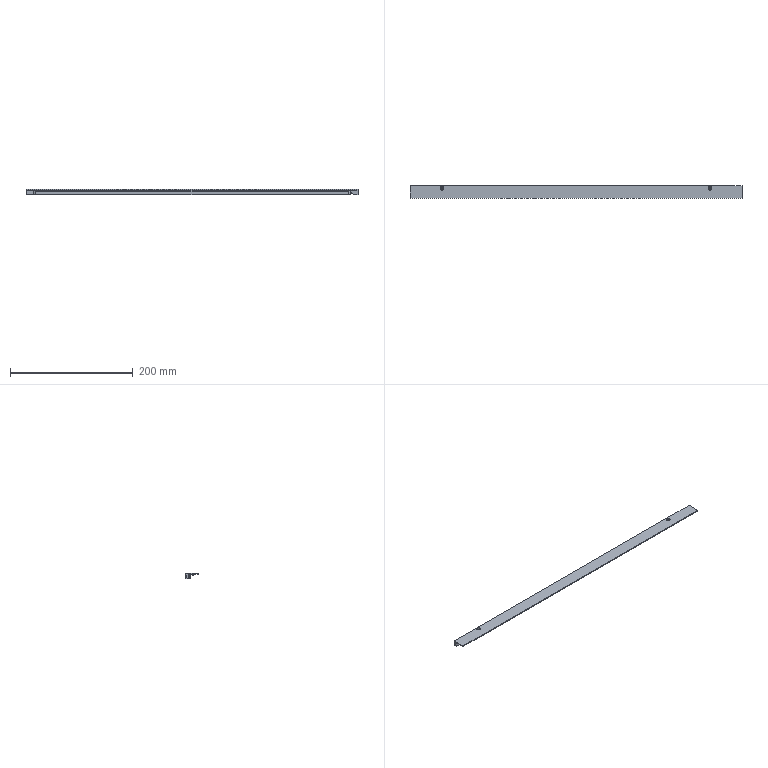Part | SolidWorks | features BaseBody 1 | 1 solid | 46 faces | box 540 x 20 x 9 mm | volume 48939 mm3 | plane 31 | cylinder 13 | cone 2 | commonest cylinder face diameters 6 x6 3.3 x4 2.076 x2 3.8 x1
STEP:
#1=CARTESIAN_POINT('',(-221.,187.,8.8));
#2=VERTEX_POINT('',#1);
#3=CARTESIAN_POINT('',(-215.,187.,8.8));
#4=VERTEX_POINT('',#3);
#5=CARTESIAN_POINT('',(-218.,187.,8.8));
#6=DIRECTION('',(0.,0.,1.));
#7=DIRECTION('',(1.,0.,0.));
#8=AXIS2_PLACEMENT_3D('',#5,#6,#7);
#9=CIRCLE('',#8,3.);
#10=EDGE_CURVE('',#2,#4,#9,.T.);
#11=ORIENTED_EDGE('',*,*,#10,.F.);
#12=CARTESIAN_POINT('',(-221.,187.,12.));
#13=VERTEX_POINT('',#12);
#14=CARTESIAN_POINT('',(-221.,187.,10.4));
#15=DIRECTION('',(0.,0.,1.));
#16=VECTOR('',#15,1000.);
#17=LINE('',#14,#16);
#18=EDGE_CURVE('',#2,#13,#17,.T.);
#19=ORIENTED_EDGE('',*,*,#18,.T.);
#20=CARTESIAN_POINT('',(-215.,187.,12.));
#21=VERTEX_POINT('',#20);
#22=CARTESIAN_POINT('',(-218.,187.,12.));
#23=DIRECTION('',(0.,0.,1.));
#24=DIRECTION('',(1.,0.,0.));
#25=AXIS2_PLACEMENT_3D('',#22,#23,#24);
#26=CIRCLE('',#25,3.);
#27=EDGE_CURVE('',#13,#21,#26,.T.);
#28=ORIENTED_EDGE('',*,*,#27,.T.);
#29=CARTESIAN_POINT('',(-215.,187.,10.4));
#30=DIRECTION('',(0.,0.,1.));
#31=VECTOR('',#30,1000.);
#32=LINE('',#29,#31);
#33=EDGE_CURVE('',#4,#21,#32,.T.);
#34=ORIENTED_EDGE('',*,*,#33,.F.);
#35=EDGE_LOOP('',(#11,#19,#28,#34));
#36=FACE_OUTER_BOUND('',#35,.T.);
#37=CARTESIAN_POINT('',(-218.,187.,10.4));
#38=DIRECTION('',(0.,0.,1.));
#39=DIRECTION('',(1.,0.,0.));
#40=AXIS2_PLACEMENT_3D('',#37,#38,#39);
#41=CYLINDRICAL_SURFACE('',#40,3.);
#42=ADVANCED_FACE('',(#36),#41,.F.);
#43=CARTESIAN_POINT('',(215.,187.,8.8));
#44=VERTEX_POINT('',#43);
#45=CARTESIAN_POINT('',(221.,187.,8.8));
#46=VERTEX_POINT('',#45);
#47=CARTESIAN_POINT('',(218.,187.,8.8));
#48=DIRECTION('',(0.,0.,1.));
#49=DIRECTION('',(1.,0.,0.));
#50=AXIS2_PLACEMENT_3D('',#47,#48,#49);
#51=CIRCLE('',#50,3.);
#52=EDGE_CURVE('',#44,#46,#51,.T.);
#53=ORIENTED_EDGE('',*,*,#52,.F.);
#54=CARTESIAN_POINT('',(215.,187.,12.));
#55=VERTEX_POINT('',#54);
#56=CARTESIAN_POINT('',(215.,187.,10.4));
#57=DIRECTION('',(0.,0.,1.));
#58=VECTOR('',#57,1000.);
#59=LINE('',#56,#58);
#60=EDGE_CURVE('',#44,#55,#59,.T.);
#61=ORIENTED_EDGE('',*,*,#60,.T.);
#62=CARTESIAN_POINT('',(221.,187.,12.));
#63=VERTEX_POINT('',#62);
#64=CARTESIAN_POINT('',(218.,187.,12.));
#65=DIRECTION('',(0.,0.,1.));
#66=DIRECTION('',(1.,0.,0.));
#67=AXIS2_PLACEMENT_3D('',#64,#65,#66);
#68=CIRCLE('',#67,3.);
#69=EDGE_CURVE('',#55,#63,#68,.T.);
#70=ORIENTED_EDGE('',*,*,#69,.T.);
#71=CARTESIAN_POINT('',(221.,187.,10.4));
#72=DIRECTION('',(0.,0.,1.));
#73=VECTOR('',#72,1000.);
#74=LINE('',#71,#73);
#75=EDGE_CURVE('',#46,#63,#74,.T.);
#76=ORIENTED_EDGE('',*,*,#75,.F.);
#77=EDGE_LOOP('',(#53,#61,#70,#76));
#78=FACE_OUTER_BOUND('',#77,.T.);
#79=CARTESIAN_POINT('',(218.,187.,10.4));
#80=DIRECTION('',(0.,0.,1.));
#81=DIRECTION('',(1.,0.,0.));
#82=AXIS2_PLACEMENT_3D('',#79,#80,#81);
#83=CYLINDRICAL_SURFACE('',#82,3.);
#84=ADVANCED_FACE('',(#78),#83,.F.);
#85=CARTESIAN_POINT('',(-216.66,186.038,6.5));
#86=VERTEX_POINT('',#85);
#87=CARTESIAN_POINT('',(-219.34,186.038,6.5));
#88=VERTEX_POINT('',#87);
#89=CARTESIAN_POINT('',(-216.66,186.038,6.5));
#90=CARTESIAN_POINT('',(-216.66,186.038,6.326));
#91=CARTESIAN_POINT('',(-216.69,185.992,6.155));
#92=CARTESIAN_POINT('',(-216.821,185.842,5.872));
#93=CARTESIAN_POINT('',(-216.923,185.74,5.764));
#94=CARTESIAN_POINT('',(-217.115,185.605,5.655));
#95=CARTESIAN_POINT('',(-217.186,185.563,5.627));
#96=CARTESIAN_POINT('',(-217.334,185.488,5.583));
#97=CARTESIAN_POINT('',(-217.412,185.456,5.567));
#98=CARTESIAN_POINT('',(-217.657,185.377,5.531));
#99=CARTESIAN_POINT('',(-217.829,185.35,5.523));
#100=CARTESIAN_POINT('',(-218.174,185.35,5.523));
#101=CARTESIAN_POINT('',(-218.345,185.377,5.532));
#102=CARTESIAN_POINT('',(-218.589,185.456,5.568));
#103=CARTESIAN_POINT('',(-218.667,185.489,5.583));
#104=CARTESIAN_POINT('',(-218.816,185.563,5.627));
#105=CARTESIAN_POINT('',(-218.887,185.606,5.656));
#106=CARTESIAN_POINT('',(-219.014,185.696,5.728));
#107=CARTESIAN_POINT('',(-219.072,185.744,5.773));
#108=CARTESIAN_POINT('',(-219.171,185.836,5.881));
#109=CARTESIAN_POINT('',(-219.212,185.879,5.943));
#110=CARTESIAN_POINT('',(-219.31,185.992,6.155));
#111=CARTESIAN_POINT('',(-219.34,186.038,6.328));
#112=CARTESIAN_POINT('',(-219.34,186.038,6.5));
#113=B_SPLINE_CURVE_WITH_KNOTS('',3,(#89,#90,#91,#92,#93,#94,#95,#96,#97,#98,#99,#100,#101,#102,#103,#104,#105,#106,#107,#108,#109,#110,#111,#112),.UNSPECIFIED.,.F.,.F.,(4,2,2,2,2,2,2,2,2,2,2,4),(0.,0.0005158,0.001032,0.00129,0.001548,0.002063,0.002579,0.002837,0.003095,0.003353,0.003611,0.004127),.UNSPECIFIED.);
#114=EDGE_CURVE('',#86,#88,#113,.T.);
#115=ORIENTED_EDGE('',*,*,#114,.F.);
#116=CARTESIAN_POINT('',(-219.34,186.038,6.5));
#117=CARTESIAN_POINT('',(-219.34,186.038,6.672));
#118=CARTESIAN_POINT('',(-219.31,185.991,6.846));
#119=CARTESIAN_POINT('',(-219.18,185.842,7.127));
#120=CARTESIAN_POINT('',(-219.077,185.741,7.236));
#121=CARTESIAN_POINT('',(-218.821,185.56,7.381));
#122=CARTESIAN_POINT('',(-218.668,185.482,7.421));
#123=CARTESIAN_POINT('',(-218.345,185.378,7.468));
#124=CARTESIAN_POINT('',(-218.172,185.35,7.477));
#125=CARTESIAN_POINT('',(-217.828,185.35,7.477));
#126=CARTESIAN_POINT('',(-217.656,185.377,7.468));
#127=CARTESIAN_POINT('',(-217.413,185.456,7.433));
#128=CARTESIAN_POINT('',(-217.333,185.488,7.417));
#129=CARTESIAN_POINT('',(-217.185,185.563,7.373));
#130=CARTESIAN_POINT('',(-217.115,185.605,7.345));
#131=CARTESIAN_POINT('',(-216.986,185.696,7.272));
#132=CARTESIAN_POINT('',(-216.929,185.743,7.228));
#133=CARTESIAN_POINT('',(-216.83,185.835,7.12));
#134=CARTESIAN_POINT('',(-216.788,185.879,7.057));
#135=CARTESIAN_POINT('',(-216.691,185.991,6.847));
#136=CARTESIAN_POINT('',(-216.66,186.038,6.674));
#137=CARTESIAN_POINT('',(-216.66,186.038,6.5));
#138=B_SPLINE_CURVE_WITH_KNOTS('',3,(#116,#117,#118,#119,#120,#121,#122,#123,#124,#125,#126,#127,#128,#129,#130,#131,#132,#133,#134,#135,#136,#137),.UNSPECIFIED.,.F.,.F.,(4,2,2,2,2,2,2,2,2,2,4),(0.004127,0.004642,0.005157,0.005672,0.006187,0.006702,0.00696,0.007217,0.007475,0.007733,0.008248),.UNSPECIFIED.);
#139=EDGE_CURVE('',#88,#86,#138,.T.);
#140=ORIENTED_EDGE('',*,*,#139,.F.);
#141=EDGE_LOOP('',(#115,#140));
#142=FACE_BOUND('',#141,.T.);
#143=CARTESIAN_POINT('',(-216.35,187.,3.));
#144=VERTEX_POINT('',#143);
#145=CARTESIAN_POINT('',(-219.65,187.,3.));
#146=VERTEX_POINT('',#145);
#147=CARTESIAN_POINT('',(-218.,187.,3.));
#148=DIRECTION('',(0.,0.,-1.));
#149=DIRECTION('',(1.,0.,0.));
#150=AXIS2_PLACEMENT_3D('',#147,#148,#149);
#151=CIRCLE('',#150,1.65);
#152=EDGE_CURVE('',#144,#146,#151,.T.);
#153=ORIENTED_EDGE('',*,*,#152,.T.);
#154=CARTESIAN_POINT('',(-219.65,187.,8.8));
#155=VERTEX_POINT('',#154);
#156=CARTESIAN_POINT('',(-219.65,187.,7.));
#157=DIRECTION('',(0.,0.,1.));
#158=VECTOR('',#157,1000.);
#159=LINE('',#156,#158);
#160=EDGE_CURVE('',#146,#155,#159,.T.);
#161=ORIENTED_EDGE('',*,*,#160,.T.);
#162=CARTESIAN_POINT('',(-216.35,187.,8.8));
#163=VERTEX_POINT('',#162);
#164=CARTESIAN_POINT('',(-218.,187.,8.8));
#165=DIRECTION('',(0.,0.,-1.));
#166=DIRECTION('',(1.,0.,0.));
#167=AXIS2_PLACEMENT_3D('',#164,#165,#166);
#168=CIRCLE('',#167,1.65);
#169=EDGE_CURVE('',#163,#155,#168,.T.);
#170=ORIENTED_EDGE('',*,*,#169,.F.);
#171=CARTESIAN_POINT('',(-216.35,187.,7.));
#172=DIRECTION('',(0.,0.,1.));
#173=VECTOR('',#172,1000.);
#174=LINE('',#171,#173);
#175=EDGE_CURVE('',#144,#163,#174,.T.);
#176=ORIENTED_EDGE('',*,*,#175,.F.);
#177=EDGE_LOOP('',(#153,#161,#170,#176));
#178=FACE_OUTER_BOUND('',#177,.T.);
#179=CARTESIAN_POINT('',(-218.,187.,7.));
#180=DIRECTION('',(0.,0.,1.));
#181=DIRECTION('',(1.,0.,0.));
#182=AXIS2_PLACEMENT_3D('',#179,#180,#181);
#183=CYLINDRICAL_SURFACE('',#182,1.65);
#184=ADVANCED_FACE('',(#142,#178),#183,.F.);
#185=CARTESIAN_POINT('',(219.65,187.,3.));
#186=VERTEX_POINT('',#185);
#187=CARTESIAN_POINT('',(216.35,187.,3.));
#188=VERTEX_POINT('',#187);
#189=CARTESIAN_POINT('',(218.,187.,3.));
#190=DIRECTION('',(0.,0.,-1.));
#191=DIRECTION('',(1.,0.,0.));
#192=AXIS2_PLACEMENT_3D('',#189,#190,#191);
#193=CIRCLE('',#192,1.65);
#194=EDGE_CURVE('',#186,#188,#193,.T.);
#195=ORIENTED_EDGE('',*,*,#194,.T.);
#196=CARTESIAN_POINT('',(216.35,187.,8.8));
#197=VERTEX_POINT('',#196);
#198=CARTESIAN_POINT('',(216.35,187.,7.));
#199=DIRECTION('',(0.,0.,1.));
#200=VECTOR('',#199,1000.);
#201=LINE('',#198,#200);
#202=EDGE_CURVE('',#188,#197,#201,.T.);
#203=ORIENTED_EDGE('',*,*,#202,.T.);
#204=CARTESIAN_POINT('',(219.65,187.,8.8));
#205=VERTEX_POINT('',#204);
#206=CARTESIAN_POINT('',(218.,187.,8.8));
#207=DIRECTION('',(0.,0.,-1.));
#208=DIRECTION('',(1.,0.,0.));
#209=AXIS2_PLACEMENT_3D('',#206,#207,#208);
#210=CIRCLE('',#209,1.65);
#211=EDGE_CURVE('',#205,#197,#210,.T.);
#212=ORIENTED_EDGE('',*,*,#211,.F.);
#213=CARTESIAN_POINT('',(219.65,187.,7.));
#214=DIRECTION('',(0.,0.,1.));
#215=VECTOR('',#214,1000.);
#216=LINE('',#213,#215);
#217=EDGE_CURVE('',#186,#205,#216,.T.);
#218=ORIENTED_EDGE('',*,*,#217,.F.);
#219=EDGE_LOOP('',(#195,#203,#212,#218));
#220=FACE_OUTER_BOUND('',#219,.T.);
#221=CARTESIAN_POINT('',(218.,187.,7.));
#222=DIRECTION('',(0.,0.,1.));
#223=DIRECTION('',(1.,0.,0.));
#224=AXIS2_PLACEMENT_3D('',#221,#222,#223);
#225=CYLINDRICAL_SURFACE('',#224,1.65);
#226=ADVANCED_FACE('',(#220),#225,.F.);
#227=CARTESIAN_POINT('',(-30.,186.038,6.5));
#228=VERTEX_POINT('',#227);
#229=CARTESIAN_POINT('',(-30.,185.,5.462));
#230=VERTEX_POINT('',#229);
#231=CARTESIAN_POINT('',(-30.,185.,6.5));
#232=DIRECTION('',(-1.,0.,0.));
#233=DIRECTION('',(0.,-1.,0.));
#234=AXIS2_PLACEMENT_3D('',#231,#232,#233);
#235=CIRCLE('',#234,1.038);
#236=EDGE_CURVE('',#228,#230,#235,.T.);
#237=ORIENTED_EDGE('',*,*,#236,.F.);
#238=CARTESIAN_POINT('',(-150.,186.038,6.5));
#239=DIRECTION('',(-1.,0.,0.));
#240=VECTOR('',#239,1000.);
#241=LINE('',#238,#240);
#242=EDGE_CURVE('',#228,#86,#241,.T.);
#243=ORIENTED_EDGE('',*,*,#242,.T.);
#244=ORIENTED_EDGE('',*,*,#114,.T.);
#245=CARTESIAN_POINT('',(-254.798,186.038,6.5));
#246=VERTEX_POINT('',#245);
#247=CARTESIAN_POINT('',(-150.,186.038,6.5));
#248=DIRECTION('',(-1.,0.,0.));
#249=VECTOR('',#248,1000.);
#250=LINE('',#247,#249);
#251=EDGE_CURVE('',#88,#246,#250,.T.);
#252=ORIENTED_EDGE('',*,*,#251,.T.);
#253=CARTESIAN_POINT('',(-254.,184.,6.223));
#254=VERTEX_POINT('',#253);
#255=CARTESIAN_POINT('',(-254.798,186.038,6.5));
#256=CARTESIAN_POINT('',(-254.798,186.038,6.368));
#257=CARTESIAN_POINT('',(-254.774,186.012,6.239));
#258=CARTESIAN_POINT('',(-254.696,185.922,6.008));
#259=CARTESIAN_POINT('',(-254.642,185.858,5.904));
#260=CARTESIAN_POINT('',(-254.472,185.627,5.641));
#261=CARTESIAN_POINT('',(-254.343,185.416,5.52));
#262=CARTESIAN_POINT('',(-254.192,185.065,5.457));
#263=CARTESIAN_POINT('',(-254.148,184.939,5.457));
#264=CARTESIAN_POINT('',(-254.078,184.694,5.501));
#265=CARTESIAN_POINT('',(-254.053,184.57,5.547));
#266=CARTESIAN_POINT('',(-254.019,184.351,5.68));
#267=CARTESIAN_POINT('',(-254.01,184.252,5.77));
#268=CARTESIAN_POINT('',(-254.,184.095,5.977));
#269=CARTESIAN_POINT('',(-254.,184.035,6.096));
#270=CARTESIAN_POINT('',(-254.,184.,6.223));
#271=B_SPLINE_CURVE_WITH_KNOTS('',3,(#255,#256,#257,#258,#259,#260,#261,#262,#263,#264,#265,#266,#267,#268,#269,#270),.UNSPECIFIED.,.F.,.F.,(4,2,2,2,2,2,2,4),(0.003112,0.003501,0.00389,0.004667,0.005056,0.005445,0.005833,0.006222),.UNSPECIFIED.);
#272=EDGE_CURVE('',#246,#254,#271,.T.);
#273=ORIENTED_EDGE('',*,*,#272,.T.);
#274=CARTESIAN_POINT('',(-254.,183.962,6.5));
#275=VERTEX_POINT('',#274);
#276=CARTESIAN_POINT('',(-254.,185.,6.5));
#277=DIRECTION('',(1.,0.,0.));
#278=DIRECTION('',(0.,-1.,0.));
#279=AXIS2_PLACEMENT_3D('',#276,#277,#278);
#280=CIRCLE('',#279,1.038);
#281=EDGE_CURVE('',#275,#254,#280,.T.);
#282=ORIENTED_EDGE('',*,*,#281,.F.);
#283=CARTESIAN_POINT('',(-30.,183.962,6.5));
#284=VERTEX_POINT('',#283);
#285=CARTESIAN_POINT('',(-150.,183.962,6.5));
#286=DIRECTION('',(-1.,0.,0.));
#287=VECTOR('',#286,1000.);
#288=LINE('',#285,#287);
#289=EDGE_CURVE('',#284,#275,#288,.T.);
#290=ORIENTED_EDGE('',*,*,#289,.F.);
#291=CARTESIAN_POINT('',(-30.,185.,6.5));
#292=DIRECTION('',(-1.,0.,0.));
#293=DIRECTION('',(0.,-1.,0.));
#294=AXIS2_PLACEMENT_3D('',#291,#292,#293);
#295=CIRCLE('',#294,1.038);
#296=EDGE_CURVE('',#230,#284,#295,.T.);
#297=ORIENTED_EDGE('',*,*,#296,.F.);
#298=EDGE_LOOP('',(#237,#243,#244,#252,#273,#282,#290,#297));
#299=FACE_OUTER_BOUND('',#298,.T.);
#300=CARTESIAN_POINT('',(-150.,185.,6.5));
#301=DIRECTION('',(-1.,0.,0.));
#302=DIRECTION('',(0.,-1.,0.));
#303=AXIS2_PLACEMENT_3D('',#300,#301,#302);
#304=CYLINDRICAL_SURFACE('',#303,1.038);
#305=ADVANCED_FACE('',(#299),#304,.F.);
#306=CARTESIAN_POINT('',(-29.376,185.,6.5));
#307=VERTEX_POINT('',#306);
#308=CARTESIAN_POINT('',(-30.,185.,7.538));
#309=VERTEX_POINT('',#308);
#310=CARTESIAN_POINT('',(-30.,185.,7.538));
#311=DIRECTION('',(-0.515,0.,0.8572));
#312=VECTOR('',#311,1000.);
#313=LINE('',#310,#312);
#314=EDGE_CURVE('',#307,#309,#313,.T.);
#315=ORIENTED_EDGE('',*,*,#314,.F.);
#316=CARTESIAN_POINT('',(-30.,185.,5.462));
#317=DIRECTION('',(-0.515,0.,-0.8572));
#318=VECTOR('',#317,1000.);
#319=LINE('',#316,#318);
#320=EDGE_CURVE('',#307,#230,#319,.T.);
#321=ORIENTED_EDGE('',*,*,#320,.T.);
#322=ORIENTED_EDGE('',*,*,#296,.T.);
#323=CARTESIAN_POINT('',(-30.,185.,6.5));
#324=DIRECTION('',(-1.,0.,0.));
#325=DIRECTION('',(0.,-1.,0.));
#326=AXIS2_PLACEMENT_3D('',#323,#324,#325);
#327=CIRCLE('',#326,1.038);
#328=EDGE_CURVE('',#284,#309,#327,.T.);
#329=ORIENTED_EDGE('',*,*,#328,.T.);
#330=EDGE_LOOP('',(#315,#321,#322,#329));
#331=FACE_OUTER_BOUND('',#330,.T.);
#332=CARTESIAN_POINT('',(-30.,185.,6.5));
#333=DIRECTION('',(-1.,0.,0.));
#334=DIRECTION('',(0.,0.,1.));
#335=AXIS2_PLACEMENT_3D('',#332,#333,#334);
#336=CONICAL_SURFACE('',#335,1.038,1.03);
#337=ADVANCED_FACE('',(#331),#336,.F.);
#338=CARTESIAN_POINT('',(-218.,187.,12.));
#339=DIRECTION('',(0.,0.,1.));
#340=DIRECTION('',(1.,0.,0.));
#341=AXIS2_PLACEMENT_3D('',#338,#339,#340);
#342=CIRCLE('',#341,3.);
#343=EDGE_CURVE('',#21,#13,#342,.T.);
#344=ORIENTED_EDGE('',*,*,#343,.F.);
#345=ORIENTED_EDGE('',*,*,#27,.F.);
#346=EDGE_LOOP('',(#344,#345));
#347=FACE_BOUND('',#346,.T.);
#348=CARTESIAN_POINT('',(218.,187.,12.));
#349=DIRECTION('',(0.,0.,1.));
#350=DIRECTION('',(1.,0.,0.));
#351=AXIS2_PLACEMENT_3D('',#348,#349,#350);
#352=CIRCLE('',#351,3.);
#353=EDGE_CURVE('',#63,#55,#352,.T.);
#354=ORIENTED_EDGE('',*,*,#353,.F.);
#355=ORIENTED_EDGE('',*,*,#69,.F.);
#356=EDGE_LOOP('',(#354,#355));
#357=FACE_BOUND('',#356,.T.);
#358=CARTESIAN_POINT('',(-270.,191.,12.));
#359=VERTEX_POINT('',#358);
#360=CARTESIAN_POINT('',(270.,191.,12.));
#361=VERTEX_POINT('',#360);
#362=CARTESIAN_POINT('',(-270.,191.,12.));
#363=DIRECTION('',(1.,0.,0.));
#364=VECTOR('',#363,1000.);
#365=LINE('',#362,#364);
#366=EDGE_CURVE('',#359,#361,#365,.T.);
#367=ORIENTED_EDGE('',*,*,#366,.F.);
#368=CARTESIAN_POINT('',(-270.,171.,12.));
#369=VERTEX_POINT('',#368);
#370=CARTESIAN_POINT('',(-270.,171.,12.));
#371=DIRECTION('',(0.,1.,0.));
#372=VECTOR('',#371,1000.);
#373=LINE('',#370,#372);
#374=EDGE_CURVE('',#369,#359,#373,.T.);
#375=ORIENTED_EDGE('',*,*,#374,.F.);
#376=CARTESIAN_POINT('',(270.,171.,12.));
#377=VERTEX_POINT('',#376);
#378=CARTESIAN_POINT('',(-270.,171.,12.));
#379=DIRECTION('',(-1.,0.,0.));
#380=VECTOR('',#379,1000.);
#381=LINE('',#378,#380);
#382=EDGE_CURVE('',#377,#369,#381,.T.);
#383=ORIENTED_EDGE('',*,*,#382,.F.);
#384=CARTESIAN_POINT('',(270.,171.,12.));
#385=DIRECTION('',(0.,-1.,0.));
#386=VECTOR('',#385,1000.);
#387=LINE('',#384,#386);
#388=EDGE_CURVE('',#361,#377,#387,.T.);
#389=ORIENTED_EDGE('',*,*,#388,.F.);
#390=EDGE_LOOP('',(#367,#375,#383,#389));
#391=FACE_OUTER_BOUND('',#390,.T.);
#392=CARTESIAN_POINT('',(-270.,171.,12.));
#393=DIRECTION('',(0.,0.,-1.));
#394=DIRECTION('',(-1.,0.,0.));
#395=AXIS2_PLACEMENT_3D('',#392,#393,#394);
#396=PLANE('',#395);
#397=ADVANCED_FACE('',(#347,#357,#391),#396,.F.);
#398=ORIENTED_EDGE('',*,*,#18,.F.);
#399=CARTESIAN_POINT('',(-218.,187.,8.8));
#400=DIRECTION('',(0.,0.,1.));
#401=DIRECTION('',(1.,0.,0.));
#402=AXIS2_PLACEMENT_3D('',#399,#400,#401);
#403=CIRCLE('',#402,3.);
#404=EDGE_CURVE('',#4,#2,#403,.T.);
#405=ORIENTED_EDGE('',*,*,#404,.F.);
#406=ORIENTED_EDGE('',*,*,#33,.T.);
#407=ORIENTED_EDGE('',*,*,#343,.T.);
#408=EDGE_LOOP('',(#398,#405,#406,#407));
#409=FACE_OUTER_BOUND('',#408,.T.);
#410=CARTESIAN_POINT('',(-218.,187.,10.4));
#411=DIRECTION('',(0.,0.,1.));
#412=DIRECTION('',(1.,0.,0.));
#413=AXIS2_PLACEMENT_3D('',#410,#411,#412);
#414=CYLINDRICAL_SURFACE('',#413,3.);
#415=ADVANCED_FACE('',(#409),#414,.F.);
#416=ORIENTED_EDGE('',*,*,#60,.F.);
#417=CARTESIAN_POINT('',(218.,187.,8.8));
#418=DIRECTION('',(0.,0.,1.));
#419=DIRECTION('',(1.,0.,0.));
#420=AXIS2_PLACEMENT_3D('',#417,#418,#419);
#421=CIRCLE('',#420,3.);
#422=EDGE_CURVE('',#46,#44,#421,.T.);
#423=ORIENTED_EDGE('',*,*,#422,.F.);
#424=ORIENTED_EDGE('',*,*,#75,.T.);
#425=ORIENTED_EDGE('',*,*,#353,.T.);
#426=EDGE_LOOP('',(#416,#423,#424,#425));
#427=FACE_OUTER_BOUND('',#426,.T.);
#428=CARTESIAN_POINT('',(218.,187.,10.4));
#429=DIRECTION('',(0.,0.,1.));
#430=DIRECTION('',(1.,0.,0.));
#431=AXIS2_PLACEMENT_3D('',#428,#429,#430);
#432=CYLINDRICAL_SURFACE('',#431,3.);
#433=ADVANCED_FACE('',(#427),#432,.F.);
#434=CARTESIAN_POINT('',(270.,190.,6.));
#435=VERTEX_POINT('',#434);
#436=CARTESIAN_POINT('',(270.,190.,4.5));
#437=VERTEX_POINT('',#436);
#438=CARTESIAN_POINT('',(270.,190.,4.5));
#439=DIRECTION('',(0.,0.,-1.));
#440=VECTOR('',#439,1000.);
#441=LINE('',#438,#440);
#442=EDGE_CURVE('',#435,#437,#441,.T.);
#443=ORIENTED_EDGE('',*,*,#442,.F.);
#444=CARTESIAN_POINT('',(270.,191.,6.));
#445=VERTEX_POINT('',#444);
#446=CARTESIAN_POINT('',(270.,190.,6.));
#447=DIRECTION('',(0.,-1.,0.));
#448=VECTOR('',#447,1000.);
#449=LINE('',#446,#448);
#450=EDGE_CURVE('',#445,#435,#449,.T.);
#451=ORIENTED_EDGE('',*,*,#450,.F.);
#452=CARTESIAN_POINT('',(270.,191.,7.));
#453=VERTEX_POINT('',#452);
#454=CARTESIAN_POINT('',(270.,191.,12.));
#455=DIRECTION('',(0.,0.,1.));
#456=VECTOR('',#455,1000.);
#457=LINE('',#454,#456);
#458=EDGE_CURVE('',#445,#453,#457,.T.);
#459=ORIENTED_EDGE('',*,*,#458,.T.);
#460=CARTESIAN_POINT('',(270.,190.,7.));
#461=VERTEX_POINT('',#460);
#462=CARTESIAN_POINT('',(270.,191.,7.));
#463=DIRECTION('',(0.,1.,0.));
#464=VECTOR('',#463,1000.);
#465=LINE('',#462,#464);
#466=EDGE_CURVE('',#461,#453,#465,.T.);
#467=ORIENTED_EDGE('',*,*,#466,.F.);
#468=CARTESIAN_POINT('',(270.,190.,8.5));
#469=VERTEX_POINT('',#468);
#470=CARTESIAN_POINT('',(270.,190.,7.));
#471=DIRECTION('',(0.,0.,-1.));
#472=VECTOR('',#471,1000.);
#473=LINE('',#470,#472);
#474=EDGE_CURVE('',#469,#461,#473,.T.);
#475=ORIENTED_EDGE('',*,*,#474,.F.);
#476=CARTESIAN_POINT('',(270.,191.,8.5));
#477=VERTEX_POINT('',#476);
#478=CARTESIAN_POINT('',(270.,190.,8.5));
#479=DIRECTION('',(0.,-1.,0.));
#480=VECTOR('',#479,1000.);
#481=LINE('',#478,#480);
#482=EDGE_CURVE('',#477,#469,#481,.T.);
#483=ORIENTED_EDGE('',*,*,#482,.F.);
#484=CARTESIAN_POINT('',(270.,191.,7.5));
#485=DIRECTION('',(0.,0.,-1.));
#486=VECTOR('',#485,1000.);
#487=LINE('',#484,#486);
#488=EDGE_CURVE('',#361,#477,#487,.T.);
#489=ORIENTED_EDGE('',*,*,#488,.F.);
#490=ORIENTED_EDGE('',*,*,#388,.T.);
#491=CARTESIAN_POINT('',(270.,171.,10.5));
#492=VERTEX_POINT('',#491);
#493=CARTESIAN_POINT('',(270.,171.,7.5));
#494=DIRECTION('',(0.,0.,1.));
#495=VECTOR('',#494,1000.);
#496=LINE('',#493,#495);
#497=EDGE_CURVE('',#492,#377,#496,.T.);
#498=ORIENTED_EDGE('',*,*,#497,.F.);
#499=CARTESIAN_POINT('',(270.,187.,10.5));
#500=VERTEX_POINT('',#499);
#501=CARTESIAN_POINT('',(270.,181.,10.5));
#502=DIRECTION('',(0.,-1.,0.));
#503=VECTOR('',#502,1000.);
#504=LINE('',#501,#503);
#505=EDGE_CURVE('',#500,#492,#504,.T.);
#506=ORIENTED_EDGE('',*,*,#505,.F.);
#507=CARTESIAN_POINT('',(270.,187.,3.));
#508=VERTEX_POINT('',#507);
#509=CARTESIAN_POINT('',(270.,187.,7.5));
#510=DIRECTION('',(0.,0.,1.));
#511=VECTOR('',#510,1000.);
#512=LINE('',#509,#511);
#513=EDGE_CURVE('',#508,#500,#512,.T.);
#514=ORIENTED_EDGE('',*,*,#513,.F.);
#515=CARTESIAN_POINT('',(270.,191.,3.));
#516=VERTEX_POINT('',#515);
#517=CARTESIAN_POINT('',(270.,181.,3.));
#518=DIRECTION('',(0.,-1.,0.));
#519=VECTOR('',#518,1000.);
#520=LINE('',#517,#519);
#521=EDGE_CURVE('',#516,#508,#520,.T.);
#522=ORIENTED_EDGE('',*,*,#521,.F.);
#523=CARTESIAN_POINT('',(270.,191.,4.5));
#524=VERTEX_POINT('',#523);
#525=CARTESIAN_POINT('',(270.,191.,12.));
#526=DIRECTION('',(0.,0.,1.));
#527=VECTOR('',#526,1000.);
#528=LINE('',#525,#527);
#529=EDGE_CURVE('',#516,#524,#528,.T.);
#530=ORIENTED_EDGE('',*,*,#529,.T.);
#531=CARTESIAN_POINT('',(270.,191.,4.5));
#532=DIRECTION('',(0.,1.,0.));
#533=VECTOR('',#532,1000.);
#534=LINE('',#531,#533);
#535=EDGE_CURVE('',#437,#524,#534,.T.);
#536=ORIENTED_EDGE('',*,*,#535,.F.);
#537=EDGE_LOOP('',(#443,#451,#459,#467,#475,#483,#489,#490,#498,#506,#514,#522,#530,#536));
#538=FACE_OUTER_BOUND('',#537,.T.);
#539=CARTESIAN_POINT('',(270.,181.,7.5));
#540=DIRECTION('',(-1.,0.,0.));
#541=DIRECTION('',(0.,-1.,0.));
#542=AXIS2_PLACEMENT_3D('',#539,#540,#541);
#543=PLANE('',#542);
#544=ADVANCED_FACE('',(#538),#543,.F.);
#545=CARTESIAN_POINT('',(-270.,191.,8.5));
#546=VERTEX_POINT('',#545);
#547=CARTESIAN_POINT('',(-270.,191.,12.));
#548=DIRECTION('',(0.,0.,-1.));
#549=VECTOR('',#548,1000.);
#550=LINE('',#547,#549);
#551=EDGE_CURVE('',#359,#546,#550,.T.);
#552=ORIENTED_EDGE('',*,*,#551,.F.);
#553=ORIENTED_EDGE('',*,*,#366,.T.);
#554=ORIENTED_EDGE('',*,*,#488,.T.);
#555=CARTESIAN_POINT('',(-270.,191.,8.5));
#556=DIRECTION('',(1.,0.,0.));
#557=VECTOR('',#556,1000.);
#558=LINE('',#555,#557);
#559=EDGE_CURVE('',#546,#477,#558,.T.);
#560=ORIENTED_EDGE('',*,*,#559,.F.);
#561=EDGE_LOOP('',(#552,#553,#554,#560));
#562=FACE_OUTER_BOUND('',#561,.T.);
#563=CARTESIAN_POINT('',(-270.,191.,12.));
#564=DIRECTION('',(0.,-1.,0.));
#565=DIRECTION('',(0.,0.,-1.));
#566=AXIS2_PLACEMENT_3D('',#563,#564,#565);
#567=PLANE('',#566);
#568=ADVANCED_FACE('',(#562),#567,.F.);
#569=CARTESIAN_POINT('',(-270.,191.,4.5));
#570=VERTEX_POINT('',#569);
#571=CARTESIAN_POINT('',(-270.,191.,3.));
#572=VERTEX_POINT('',#571);
#573=CARTESIAN_POINT('',(-270.,191.,12.));
#574=DIRECTION('',(0.,0.,-1.));
#575=VECTOR('',#574,1000.);
#576=LINE('',#573,#575);
#577=EDGE_CURVE('',#570,#572,#576,.T.);
#578=ORIENTED_EDGE('',*,*,#577,.T.);
#579=CARTESIAN_POINT('',(-270.,187.,3.));
#580=VERTEX_POINT('',#579);
#581=CARTESIAN_POINT('',(-270.,181.,3.));
#582=DIRECTION('',(0.,1.,0.));
#583=VECTOR('',#582,1000.);
#584=LINE('',#581,#583);
#585=EDGE_CURVE('',#580,#572,#584,.T.);
#586=ORIENTED_EDGE('',*,*,#585,.F.);
#587=CARTESIAN_POINT('',(-270.,187.,10.5));
#588=VERTEX_POINT('',#587);
#589=CARTESIAN_POINT('',(-270.,187.,7.5));
#590=DIRECTION('',(0.,0.,-1.));
#591=VECTOR('',#590,1000.);
#592=LINE('',#589,#591);
#593=EDGE_CURVE('',#588,#580,#592,.T.);
#594=ORIENTED_EDGE('',*,*,#593,.F.);
#595=CARTESIAN_POINT('',(-270.,171.,10.5));
#596=VERTEX_POINT('',#595);
#597=CARTESIAN_POINT('',(-270.,181.,10.5));
#598=DIRECTION('',(0.,1.,0.));
#599=VECTOR('',#598,1000.);
#600=LINE('',#597,#599);
#601=EDGE_CURVE('',#596,#588,#600,.T.);
#602=ORIENTED_EDGE('',*,*,#601,.F.);
#603=CARTESIAN_POINT('',(-270.,171.,7.5));
#604=DIRECTION('',(0.,0.,-1.));
#605=VECTOR('',#604,1000.);
#606=LINE('',#603,#605);
#607=EDGE_CURVE('',#369,#596,#606,.T.);
#608=ORIENTED_EDGE('',*,*,#607,.F.);
#609=ORIENTED_EDGE('',*,*,#374,.T.);
#610=ORIENTED_EDGE('',*,*,#551,.T.);
#611=CARTESIAN_POINT('',(-270.,190.,8.5));
#612=VERTEX_POINT('',#611);
#613=CARTESIAN_POINT('',(-270.,181.,8.5));
#614=DIRECTION('',(0.,1.,0.));
#615=VECTOR('',#614,1000.);
#616=LINE('',#613,#615);
#617=EDGE_CURVE('',#612,#546,#616,.T.);
#618=ORIENTED_EDGE('',*,*,#617,.F.);
#619=CARTESIAN_POINT('',(-270.,190.,7.));
#620=VERTEX_POINT('',#619);
#621=CARTESIAN_POINT('',(-270.,190.,7.));
#622=DIRECTION('',(0.,0.,1.));
#623=VECTOR('',#622,1000.);
#624=LINE('',#621,#623);
#625=EDGE_CURVE('',#620,#612,#624,.T.);
#626=ORIENTED_EDGE('',*,*,#625,.F.);
#627=CARTESIAN_POINT('',(-270.,191.,7.));
#628=VERTEX_POINT('',#627);
#629=CARTESIAN_POINT('',(-270.,191.,7.));
#630=DIRECTION('',(0.,-1.,0.));
#631=VECTOR('',#630,1000.);
#632=LINE('',#629,#631);
#633=EDGE_CURVE('',#628,#620,#632,.T.);
#634=ORIENTED_EDGE('',*,*,#633,.F.);
#635=CARTESIAN_POINT('',(-270.,191.,6.));
#636=VERTEX_POINT('',#635);
#637=CARTESIAN_POINT('',(-270.,191.,12.));
#638=DIRECTION('',(0.,0.,-1.));
#639=VECTOR('',#638,1000.);
#640=LINE('',#637,#639);
#641=EDGE_CURVE('',#628,#636,#640,.T.);
#642=ORIENTED_EDGE('',*,*,#641,.T.);
#643=CARTESIAN_POINT('',(-270.,190.,6.));
#644=VERTEX_POINT('',#643);
#645=CARTESIAN_POINT('',(-270.,190.,6.));
#646=DIRECTION('',(0.,1.,0.));
#647=VECTOR('',#646,1000.);
#648=LINE('',#645,#647);
#649=EDGE_CURVE('',#644,#636,#648,.T.);
#650=ORIENTED_EDGE('',*,*,#649,.F.);
#651=CARTESIAN_POINT('',(-270.,190.,4.5));
#652=VERTEX_POINT('',#651);
#653=CARTESIAN_POINT('',(-270.,190.,4.5));
#654=DIRECTION('',(0.,0.,1.));
#655=VECTOR('',#654,1000.);
#656=LINE('',#653,#655);
#657=EDGE_CURVE('',#652,#644,#656,.T.);
#658=ORIENTED_EDGE('',*,*,#657,.F.);
#659=CARTESIAN_POINT('',(-270.,191.,4.5));
#660=DIRECTION('',(0.,-1.,0.));
#661=VECTOR('',#660,1000.);
#662=LINE('',#659,#661);
#663=EDGE_CURVE('',#570,#652,#662,.T.);
#664=ORIENTED_EDGE('',*,*,#663,.F.);
#665=EDGE_LOOP('',(#578,#586,#594,#602,#608,#609,#610,#618,#626,#634,#642,#650,#658,#664));
#666=FACE_OUTER_BOUND('',#665,.T.);
#667=CARTESIAN_POINT('',(-270.,181.,7.5));
#668=DIRECTION('',(1.,0.,0.));
#669=DIRECTION('',(0.,1.,0.));
#670=AXIS2_PLACEMENT_3D('',#667,#668,#669);
#671=PLANE('',#670);
#672=ADVANCED_FACE('',(#666),#671,.F.);
#673=ORIENTED_EDGE('',*,*,#382,.T.);
#674=ORIENTED_EDGE('',*,*,#607,.T.);
#675=CARTESIAN_POINT('',(-270.,171.,10.5));
#676=DIRECTION('',(-1.,0.,0.));
#677=VECTOR('',#676,1000.);
#678=LINE('',#675,#677);
#679=EDGE_CURVE('',#492,#596,#678,.T.);
#680=ORIENTED_EDGE('',*,*,#679,.F.);
#681=ORIENTED_EDGE('',*,*,#497,.T.);
#682=EDGE_LOOP('',(#673,#674,#680,#681));
#683=FACE_OUTER_BOUND('',#682,.T.);
#684=CARTESIAN_POINT('',(-270.,171.,10.5));
#685=DIRECTION('',(0.,1.,0.));
#686=DIRECTION('',(0.,0.,1.));
#687=AXIS2_PLACEMENT_3D('',#684,#685,#686);
#688=PLANE('',#687);
#689=ADVANCED_FACE('',(#683),#688,.F.);
#690=ORIENTED_EDGE('',*,*,#169,.T.);
#691=CARTESIAN_POINT('',(-218.,187.,8.8));
#692=DIRECTION('',(0.,0.,-1.));
#693=DIRECTION('',(1.,0.,0.));
#694=AXIS2_PLACEMENT_3D('',#691,#692,#693);
#695=CIRCLE('',#694,1.65);
#696=EDGE_CURVE('',#155,#163,#695,.T.);
#697=ORIENTED_EDGE('',*,*,#696,.T.);
#698=EDGE_LOOP('',(#690,#697));
#699=FACE_BOUND('',#698,.T.);
#700=ORIENTED_EDGE('',*,*,#404,.T.);
#701=ORIENTED_EDGE('',*,*,#10,.T.);
#702=EDGE_LOOP('',(#700,#701));
#703=FACE_OUTER_BOUND('',#702,.T.);
#704=CARTESIAN_POINT('',(-218.,187.,8.8));
#705=DIRECTION('',(0.,0.,1.));
#706=DIRECTION('',(1.,0.,0.));
#707=AXIS2_PLACEMENT_3D('',#704,#705,#706);
#708=PLANE('',#707);
#709=ADVANCED_FACE('',(#699,#703),#708,.T.);
#710=ORIENTED_EDGE('',*,*,#211,.T.);
#711=CARTESIAN_POINT('',(218.,187.,8.8));
#712=DIRECTION('',(0.,0.,-1.));
#713=DIRECTION('',(1.,0.,0.));
#714=AXIS2_PLACEMENT_3D('',#711,#712,#713);
#715=CIRCLE('',#714,1.65);
#716=EDGE_CURVE('',#197,#205,#715,.T.);
#717=ORIENTED_EDGE('',*,*,#716,.T.);
#718=EDGE_LOOP('',(#710,#717));
#719=FACE_BOUND('',#718,.T.);
#720=ORIENTED_EDGE('',*,*,#422,.T.);
#721=ORIENTED_EDGE('',*,*,#52,.T.);
#722=EDGE_LOOP('',(#720,#721));
#723=FACE_OUTER_BOUND('',#722,.T.);
#724=CARTESIAN_POINT('',(218.,187.,8.8));
#725=DIRECTION('',(0.,0.,1.));
#726=DIRECTION('',(1.,0.,0.));
#727=AXIS2_PLACEMENT_3D('',#724,#725,#726);
#728=PLANE('',#727);
#729=ADVANCED_FACE('',(#719,#723),#728,.T.);
#730=CARTESIAN_POINT('',(254.,184.,10.5));
#731=VERTEX_POINT('',#730);
#732=CARTESIAN_POINT('',(254.,178.3,10.5));
#733=VERTEX_POINT('',#732);
#734=CARTESIAN_POINT('',(254.,178.3,10.5));
#735=DIRECTION('',(0.,-1.,0.));
#736=VECTOR('',#735,1000.);
#737=LINE('',#734,#736);
#738=EDGE_CURVE('',#731,#733,#737,.T.);
#739=ORIENTED_EDGE('',*,*,#738,.F.);
#740=CARTESIAN_POINT('',(257.,187.,10.5));
#741=VERTEX_POINT('',#740);
#742=CARTESIAN_POINT('',(257.,184.,10.5));
#743=DIRECTION('',(0.,0.,1.));
#744=DIRECTION('',(-1.,0.,0.));
#745=AXIS2_PLACEMENT_3D('',#742,#743,#744);
#746=CIRCLE('',#745,3.);
#747=EDGE_CURVE('',#741,#731,#746,.T.);
#748=ORIENTED_EDGE('',*,*,#747,.F.);
#749=CARTESIAN_POINT('',(-270.,187.,10.5));
#750=DIRECTION('',(-1.,0.,0.));
#751=VECTOR('',#750,1000.);
#752=LINE('',#749,#751);
#753=EDGE_CURVE('',#500,#741,#752,.T.);
#754=ORIENTED_EDGE('',*,*,#753,.F.);
#755=ORIENTED_EDGE('',*,*,#505,.T.);
#756=ORIENTED_EDGE('',*,*,#679,.T.);
#757=ORIENTED_EDGE('',*,*,#601,.T.);
#758=CARTESIAN_POINT('',(-257.,187.,10.5));
#759=VERTEX_POINT('',#758);
#760=CARTESIAN_POINT('',(-270.,187.,10.5));
#761=DIRECTION('',(-1.,0.,0.));
#762=VECTOR('',#761,1000.);
#763=LINE('',#760,#762);
#764=EDGE_CURVE('',#759,#588,#763,.T.);
#765=ORIENTED_EDGE('',*,*,#764,.F.);
#766=CARTESIAN_POINT('',(-254.,184.,10.5));
#767=VERTEX_POINT('',#766);
#768=CARTESIAN_POINT('',(-257.,184.,10.5));
#769=DIRECTION('',(0.,0.,1.));
#770=DIRECTION('',(-1.,0.,0.));
#771=AXIS2_PLACEMENT_3D('',#768,#769,#770);
#772=CIRCLE('',#771,3.);
#773=EDGE_CURVE('',#767,#759,#772,.T.);
#774=ORIENTED_EDGE('',*,*,#773,.F.);
#775=CARTESIAN_POINT('',(-254.,178.3,10.5));
#776=VERTEX_POINT('',#775);
#777=CARTESIAN_POINT('',(-254.,178.3,10.5));
#778=DIRECTION('',(0.,1.,0.));
#779=VECTOR('',#778,1000.);
#780=LINE('',#777,#779);
#781=EDGE_CURVE('',#776,#767,#780,.T.);
#782=ORIENTED_EDGE('',*,*,#781,.F.);
#783=CARTESIAN_POINT('',(-270.,178.3,10.5));
#784=DIRECTION('',(-1.,0.,0.));
#785=VECTOR('',#784,1000.);
#786=LINE('',#783,#785);
#787=EDGE_CURVE('',#733,#776,#786,.T.);
#788=ORIENTED_EDGE('',*,*,#787,.F.);
#789=EDGE_LOOP('',(#739,#748,#754,#755,#756,#757,#765,#774,#782,#788));
#790=FACE_OUTER_BOUND('',#789,.T.);
#791=CARTESIAN_POINT('',(-270.,178.3,10.5));
#792=DIRECTION('',(0.,0.,1.));
#793=DIRECTION('',(0.,-1.,0.));
#794=AXIS2_PLACEMENT_3D('',#791,#792,#793);
#795=PLANE('',#794);
#796=ADVANCED_FACE('',(#790),#795,.F.);
#797=CARTESIAN_POINT('',(258.1,187.,3.));
#798=VERTEX_POINT('',#797);
#799=CARTESIAN_POINT('',(258.1,187.,4.));
#800=VERTEX_POINT('',#799);
#801=CARTESIAN_POINT('',(258.1,187.,4.));
#802=DIRECTION('',(0.,0.,1.));
#803=VECTOR('',#802,1000.);
#804=LINE('',#801,#803);
#805=EDGE_CURVE('',#798,#800,#804,.T.);
#806=ORIENTED_EDGE('',*,*,#805,.T.);
#807=CARTESIAN_POINT('',(261.9,187.,4.));
#808=VERTEX_POINT('',#807);
#809=CARTESIAN_POINT('',(260.,187.,4.));
#810=DIRECTION('',(0.,1.,0.));
#811=DIRECTION('',(0.,0.,-1.));
#812=AXIS2_PLACEMENT_3D('',#809,#810,#811);
#813=CIRCLE('',#812,1.9);
#814=EDGE_CURVE('',#800,#808,#813,.T.);
#815=ORIENTED_EDGE('',*,*,#814,.T.);
#816=CARTESIAN_POINT('',(261.9,187.,3.));
#817=VERTEX_POINT('',#816);
#818=CARTESIAN_POINT('',(261.9,187.,0.));
#819=DIRECTION('',(0.,0.,-1.));
#820=VECTOR('',#819,1000.);
#821=LINE('',#818,#820);
#822=EDGE_CURVE('',#808,#817,#821,.T.);
#823=ORIENTED_EDGE('',*,*,#822,.T.);
#824=CARTESIAN_POINT('',(257.,187.,3.));
#825=DIRECTION('',(1.,0.,0.));
#826=VECTOR('',#825,1000.);
#827=LINE('',#824,#826);
#828=EDGE_CURVE('',#817,#508,#827,.T.);
#829=ORIENTED_EDGE('',*,*,#828,.T.);
#830=ORIENTED_EDGE('',*,*,#513,.T.);
#831=ORIENTED_EDGE('',*,*,#753,.T.);
#832=CARTESIAN_POINT('',(257.,187.,3.));
#833=VERTEX_POINT('',#832);
#834=CARTESIAN_POINT('',(257.,187.,3.));
#835=DIRECTION('',(0.,0.,-1.));
#836=VECTOR('',#835,1000.);
#837=LINE('',#834,#836);
#838=EDGE_CURVE('',#741,#833,#837,.T.);
#839=ORIENTED_EDGE('',*,*,#838,.T.);
#840=CARTESIAN_POINT('',(257.,187.,3.));
#841=DIRECTION('',(1.,0.,0.));
#842=VECTOR('',#841,1000.);
#843=LINE('',#840,#842);
#844=EDGE_CURVE('',#833,#798,#843,.T.);
#845=ORIENTED_EDGE('',*,*,#844,.T.);
#846=EDGE_LOOP('',(#806,#815,#823,#829,#830,#831,#839,#845));
#847=FACE_OUTER_BOUND('',#846,.T.);
#848=CARTESIAN_POINT('',(257.,187.,3.));
#849=DIRECTION('',(0.,-1.,0.));
#850=DIRECTION('',(0.,0.,-1.));
#851=AXIS2_PLACEMENT_3D('',#848,#849,#850);
#852=PLANE('',#851);
#853=ADVANCED_FACE('',(#847),#852,.T.);
#854=CARTESIAN_POINT('',(261.9,191.,3.));
#855=VERTEX_POINT('',#854);
#856=CARTESIAN_POINT('',(-270.,191.,3.));
#857=DIRECTION('',(-1.,0.,0.));
#858=VECTOR('',#857,1000.);
#859=LINE('',#856,#858);
#860=EDGE_CURVE('',#516,#855,#859,.T.);
#861=ORIENTED_EDGE('',*,*,#860,.F.);
#862=ORIENTED_EDGE('',*,*,#521,.T.);
#863=ORIENTED_EDGE('',*,*,#828,.F.);
#864=CARTESIAN_POINT('',(261.9,191.,3.));
#865=DIRECTION('',(0.,-1.,0.));
#866=VECTOR('',#865,1000.);
#867=LINE('',#864,#866);
#868=EDGE_CURVE('',#855,#817,#867,.T.);
#869=ORIENTED_EDGE('',*,*,#868,.F.);
#870=EDGE_LOOP('',(#861,#862,#863,#869));
#871=FACE_OUTER_BOUND('',#870,.T.);
#872=CARTESIAN_POINT('',(-270.,191.,3.));
#873=DIRECTION('',(0.,0.,1.));
#874=DIRECTION('',(1.,0.,0.));
#875=AXIS2_PLACEMENT_3D('',#872,#873,#874);
#876=PLANE('',#875);
#877=ADVANCED_FACE('',(#871),#876,.F.);
#878=ORIENTED_EDGE('',*,*,#617,.T.);
#879=ORIENTED_EDGE('',*,*,#559,.T.);
#880=ORIENTED_EDGE('',*,*,#482,.T.);
#881=CARTESIAN_POINT('',(-270.,190.,8.5));
#882=DIRECTION('',(-1.,0.,0.));
#883=VECTOR('',#882,1000.);
#884=LINE('',#881,#883);
#885=EDGE_CURVE('',#469,#612,#884,.T.);
#886=ORIENTED_EDGE('',*,*,#885,.T.);
#887=EDGE_LOOP('',(#878,#879,#880,#886));
#888=FACE_OUTER_BOUND('',#887,.T.);
#889=CARTESIAN_POINT('',(-270.,190.,8.5));
#890=DIRECTION('',(0.,0.,-1.));
#891=DIRECTION('',(-1.,0.,0.));
#892=AXIS2_PLACEMENT_3D('',#889,#890,#891);
#893=PLANE('',#892);
#894=ADVANCED_FACE('',(#888),#893,.T.);
#895=ORIENTED_EDGE('',*,*,#152,.F.);
#896=CARTESIAN_POINT('',(-218.,187.,3.));
#897=DIRECTION('',(0.,0.,-1.));
#898=DIRECTION('',(1.,0.,0.));
#899=AXIS2_PLACEMENT_3D('',#896,#897,#898);
#900=CIRCLE('',#899,1.65);
#901=EDGE_CURVE('',#146,#144,#900,.T.);
#902=ORIENTED_EDGE('',*,*,#901,.F.);
#903=EDGE_LOOP('',(#895,#902));
#904=FACE_BOUND('',#903,.T.);
#905=ORIENTED_EDGE('',*,*,#194,.F.);
#906=CARTESIAN_POINT('',(218.,187.,3.));
#907=DIRECTION('',(0.,0.,-1.));
#908=DIRECTION('',(1.,0.,0.));
#909=AXIS2_PLACEMENT_3D('',#906,#907,#908);
#910=CIRCLE('',#909,1.65);
#911=EDGE_CURVE('',#188,#186,#910,.T.);
#912=ORIENTED_EDGE('',*,*,#911,.F.);
#913=EDGE_LOOP('',(#905,#912));
#914=FACE_BOUND('',#913,.T.);
#915=ORIENTED_EDGE('',*,*,#844,.F.);
#916=CARTESIAN_POINT('',(254.,184.,3.));
#917=VERTEX_POINT('',#916);
#918=CARTESIAN_POINT('',(257.,184.,3.));
#919=DIRECTION('',(0.,0.,-1.));
#920=DIRECTION('',(-1.,0.,0.));
#921=AXIS2_PLACEMENT_3D('',#918,#919,#920);
#922=CIRCLE('',#921,3.);
#923=EDGE_CURVE('',#917,#833,#922,.T.);
#924=ORIENTED_EDGE('',*,*,#923,.F.);
#925=CARTESIAN_POINT('',(254.,183.,3.));
#926=VERTEX_POINT('',#925);
#927=CARTESIAN_POINT('',(254.,191.,3.));
#928=DIRECTION('',(0.,1.,0.));
#929=VECTOR('',#928,1000.);
#930=LINE('',#927,#929);
#931=EDGE_CURVE('',#926,#917,#930,.T.);
#932=ORIENTED_EDGE('',*,*,#931,.F.);
#933=CARTESIAN_POINT('',(-254.,183.,3.));
#934=VERTEX_POINT('',#933);
#935=CARTESIAN_POINT('',(-270.,183.,3.));
#936=DIRECTION('',(1.,0.,0.));
#937=VECTOR('',#936,1000.);
#938=LINE('',#935,#937);
#939=EDGE_CURVE('',#934,#926,#938,.T.);
#940=ORIENTED_EDGE('',*,*,#939,.F.);
#941=CARTESIAN_POINT('',(-254.,184.,3.));
#942=VERTEX_POINT('',#941);
#943=CARTESIAN_POINT('',(-254.,191.,3.));
#944=DIRECTION('',(0.,-1.,0.));
#945=VECTOR('',#944,1000.);
#946=LINE('',#943,#945);
#947=EDGE_CURVE('',#942,#934,#946,.T.);
#948=ORIENTED_EDGE('',*,*,#947,.F.);
#949=CARTESIAN_POINT('',(-257.,187.,3.));
#950=VERTEX_POINT('',#949);
#951=CARTESIAN_POINT('',(-257.,184.,3.));
#952=DIRECTION('',(0.,0.,-1.));
#953=DIRECTION('',(-1.,0.,0.));
#954=AXIS2_PLACEMENT_3D('',#951,#952,#953);
#955=CIRCLE('',#954,3.);
#956=EDGE_CURVE('',#950,#942,#955,.T.);
#957=ORIENTED_EDGE('',*,*,#956,.F.);
#958=CARTESIAN_POINT('',(-270.,187.,3.));
#959=DIRECTION('',(1.,0.,0.));
#960=VECTOR('',#959,1000.);
#961=LINE('',#958,#960);
#962=EDGE_CURVE('',#580,#950,#961,.T.);
#963=ORIENTED_EDGE('',*,*,#962,.F.);
#964=ORIENTED_EDGE('',*,*,#585,.T.);
#965=CARTESIAN_POINT('',(258.1,191.,3.));
#966=VERTEX_POINT('',#965);
#967=CARTESIAN_POINT('',(-270.,191.,3.));
#968=DIRECTION('',(-1.,0.,0.));
#969=VECTOR('',#968,1000.);
#970=LINE('',#967,#969);
#971=EDGE_CURVE('',#966,#572,#970,.T.);
#972=ORIENTED_EDGE('',*,*,#971,.F.);
#973=CARTESIAN_POINT('',(258.1,191.,3.));
#974=DIRECTION('',(0.,1.,0.));
#975=VECTOR('',#974,1000.);
#976=LINE('',#973,#975);
#977=EDGE_CURVE('',#798,#966,#976,.T.);
#978=ORIENTED_EDGE('',*,*,#977,.F.);
#979=EDGE_LOOP('',(#915,#924,#932,#940,#948,#957,#963,#964,#972,#978));
#980=FACE_OUTER_BOUND('',#979,.T.);
#981=CARTESIAN_POINT('',(-270.,191.,3.));
#982=DIRECTION('',(0.,0.,1.));
#983=DIRECTION('',(1.,0.,0.));
#984=AXIS2_PLACEMENT_3D('',#981,#982,#983);
#985=PLANE('',#984);
#986=ADVANCED_FACE('',(#904,#914,#980),#985,.F.);
#987=ORIENTED_EDGE('',*,*,#764,.T.);
#988=ORIENTED_EDGE('',*,*,#593,.T.);
#989=ORIENTED_EDGE('',*,*,#962,.T.);
#990=CARTESIAN_POINT('',(-257.,187.,3.));
#991=DIRECTION('',(0.,0.,1.));
#992=VECTOR('',#991,1000.);
#993=LINE('',#990,#992);
#994=EDGE_CURVE('',#950,#759,#993,.T.);
#995=ORIENTED_EDGE('',*,*,#994,.T.);
#996=EDGE_LOOP('',(#987,#988,#989,#995));
#997=FACE_OUTER_BOUND('',#996,.T.);
#998=CARTESIAN_POINT('',(-270.,187.,3.));
#999=DIRECTION('',(0.,-1.,0.));
#1000=DIRECTION('',(0.,0.,-1.));
#1001=AXIS2_PLACEMENT_3D('',#998,#999,#1000);
#1002=PLANE('',#1001);
#1003=ADVANCED_FACE('',(#997),#1002,.T.);
#1004=ORIENTED_EDGE('',*,*,#160,.F.);
#1005=ORIENTED_EDGE('',*,*,#901,.T.);
#1006=ORIENTED_EDGE('',*,*,#175,.T.);
#1007=ORIENTED_EDGE('',*,*,#696,.F.);
#1008=EDGE_LOOP('',(#1004,#1005,#1006,#1007));
#1009=FACE_OUTER_BOUND('',#1008,.T.);
#1010=CARTESIAN_POINT('',(-218.,187.,7.));
#1011=DIRECTION('',(0.,0.,1.));
#1012=DIRECTION('',(1.,0.,0.));
#1013=AXIS2_PLACEMENT_3D('',#1010,#1011,#1012);
#1014=CYLINDRICAL_SURFACE('',#1013,1.65);
#1015=ADVANCED_FACE('',(#1009),#1014,.F.);
#1016=ORIENTED_EDGE('',*,*,#202,.F.);
#1017=ORIENTED_EDGE('',*,*,#911,.T.);
#1018=ORIENTED_EDGE('',*,*,#217,.T.);
#1019=ORIENTED_EDGE('',*,*,#716,.F.);
#1020=EDGE_LOOP('',(#1016,#1017,#1018,#1019));
#1021=FACE_OUTER_BOUND('',#1020,.T.);
#1022=CARTESIAN_POINT('',(218.,187.,7.));
#1023=DIRECTION('',(0.,0.,1.));
#1024=DIRECTION('',(1.,0.,0.));
#1025=AXIS2_PLACEMENT_3D('',#1022,#1023,#1024);
#1026=CYLINDRICAL_SURFACE('',#1025,1.65);
#1027=ADVANCED_FACE('',(#1021),#1026,.F.);
#1028=ORIENTED_EDGE('',*,*,#787,.T.);
#1029=CARTESIAN_POINT('',(-254.,178.3,8.5));
#1030=VERTEX_POINT('',#1029);
#1031=CARTESIAN_POINT('',(-254.,178.3,8.5));
#1032=DIRECTION('',(0.,0.,1.));
#1033=VECTOR('',#1032,1000.);
#1034=LINE('',#1031,#1033);
#1035=EDGE_CURVE('',#1030,#776,#1034,.T.);
#1036=ORIENTED_EDGE('',*,*,#1035,.F.);
#1037=CARTESIAN_POINT('',(254.,178.3,8.5));
#1038=VERTEX_POINT('',#1037);
#1039=CARTESIAN_POINT('',(-270.,178.3,8.5));
#1040=DIRECTION('',(-1.,0.,0.));
#1041=VECTOR('',#1040,1000.);
#1042=LINE('',#1039,#1041);
#1043=EDGE_CURVE('',#1038,#1030,#1042,.T.);
#1044=ORIENTED_EDGE('',*,*,#1043,.F.);
#1045=CARTESIAN_POINT('',(254.,178.3,8.5));
#1046=DIRECTION('',(0.,0.,-1.));
#1047=VECTOR('',#1046,1000.);
#1048=LINE('',#1045,#1047);
#1049=EDGE_CURVE('',#733,#1038,#1048,.T.);
#1050=ORIENTED_EDGE('',*,*,#1049,.F.);
#1051=EDGE_LOOP('',(#1028,#1036,#1044,#1050));
#1052=FACE_OUTER_BOUND('',#1051,.T.);
#1053=CARTESIAN_POINT('',(-270.,178.3,8.5));
#1054=DIRECTION('',(0.,1.,0.));
#1055=DIRECTION('',(0.,0.,1.));
#1056=AXIS2_PLACEMENT_3D('',#1053,#1054,#1055);
#1057=PLANE('',#1056);
#1058=ADVANCED_FACE('',(#1052),#1057,.F.);
#1059=CARTESIAN_POINT('',(254.,179.8,8.5));
#1060=VERTEX_POINT('',#1059);
#1061=CARTESIAN_POINT('',(254.,179.8,9.));
#1062=VERTEX_POINT('',#1061);
#1063=CARTESIAN_POINT('',(254.,179.8,9.));
#1064=DIRECTION('',(0.,0.,1.));
#1065=VECTOR('',#1064,1000.);
#1066=LINE('',#1063,#1065);
#1067=EDGE_CURVE('',#1060,#1062,#1066,.T.);
#1068=ORIENTED_EDGE('',*,*,#1067,.T.);
#1069=CARTESIAN_POINT('',(254.,183.,9.));
#1070=VERTEX_POINT('',#1069);
#1071=CARTESIAN_POINT('',(254.,171.,9.));
#1072=DIRECTION('',(0.,1.,0.));
#1073=VECTOR('',#1072,1000.);
#1074=LINE('',#1071,#1073);
#1075=EDGE_CURVE('',#1062,#1070,#1074,.T.);
#1076=ORIENTED_EDGE('',*,*,#1075,.T.);
#1077=CARTESIAN_POINT('',(254.,183.,3.));
#1078=DIRECTION('',(0.,0.,-1.));
#1079=VECTOR('',#1078,1000.);
#1080=LINE('',#1077,#1079);
#1081=EDGE_CURVE('',#1070,#926,#1080,.T.);
#1082=ORIENTED_EDGE('',*,*,#1081,.T.);
#1083=ORIENTED_EDGE('',*,*,#931,.T.);
#1084=CARTESIAN_POINT('',(254.,184.,3.));
#1085=DIRECTION('',(0.,0.,1.));
#1086=VECTOR('',#1085,1000.);
#1087=LINE('',#1084,#1086);
#1088=EDGE_CURVE('',#917,#731,#1087,.T.);
#1089=ORIENTED_EDGE('',*,*,#1088,.T.);
#1090=ORIENTED_EDGE('',*,*,#738,.T.);
#1091=ORIENTED_EDGE('',*,*,#1049,.T.);
#1092=CARTESIAN_POINT('',(254.,171.,8.5));
#1093=DIRECTION('',(0.,1.,0.));
#1094=VECTOR('',#1093,1000.);
#1095=LINE('',#1092,#1094);
#1096=EDGE_CURVE('',#1038,#1060,#1095,.T.);
#1097=ORIENTED_EDGE('',*,*,#1096,.T.);
#1098=EDGE_LOOP('',(#1068,#1076,#1082,#1083,#1089,#1090,#1091,#1097));
#1099=FACE_OUTER_BOUND('',#1098,.T.);
#1100=CARTESIAN_POINT('',(254.,171.,3.));
#1101=DIRECTION('',(1.,0.,0.));
#1102=DIRECTION('',(0.,1.,0.));
#1103=AXIS2_PLACEMENT_3D('',#1100,#1101,#1102);
#1104=PLANE('',#1103);
#1105=ADVANCED_FACE('',(#1099),#1104,.T.);
#1106=ORIENTED_EDGE('',*,*,#838,.F.);
#1107=ORIENTED_EDGE('',*,*,#747,.T.);
#1108=ORIENTED_EDGE('',*,*,#1088,.F.);
#1109=ORIENTED_EDGE('',*,*,#923,.T.);
#1110=EDGE_LOOP('',(#1106,#1107,#1108,#1109));
#1111=FACE_OUTER_BOUND('',#1110,.T.);
#1112=CARTESIAN_POINT('',(257.,184.,3.));
#1113=DIRECTION('',(0.,0.,-1.));
#1114=DIRECTION('',(-1.,0.,0.));
#1115=AXIS2_PLACEMENT_3D('',#1112,#1113,#1114);
#1116=CYLINDRICAL_SURFACE('',#1115,3.);
#1117=ADVANCED_FACE('',(#1111),#1116,.F.);
#1118=CARTESIAN_POINT('',(-254.,184.,6.777));
#1119=VERTEX_POINT('',#1118);
#1120=CARTESIAN_POINT('',(-254.,184.,3.));
#1121=DIRECTION('',(0.,0.,-1.));
#1122=VECTOR('',#1121,1000.);
#1123=LINE('',#1120,#1122);
#1124=EDGE_CURVE('',#767,#1119,#1123,.T.);
#1125=ORIENTED_EDGE('',*,*,#1124,.F.);
#1126=ORIENTED_EDGE('',*,*,#773,.T.);
#1127=ORIENTED_EDGE('',*,*,#994,.F.);
#1128=ORIENTED_EDGE('',*,*,#956,.T.);
#1129=CARTESIAN_POINT('',(-254.,184.,3.));
#1130=DIRECTION('',(0.,0.,-1.));
#1131=VECTOR('',#1130,1000.);
#1132=LINE('',#1129,#1131);
#1133=EDGE_CURVE('',#254,#942,#1132,.T.);
#1134=ORIENTED_EDGE('',*,*,#1133,.F.);
#1135=ORIENTED_EDGE('',*,*,#272,.F.);
#1136=CARTESIAN_POINT('',(-254.,184.,6.777));
#1137=CARTESIAN_POINT('',(-254.,184.035,6.904));
#1138=CARTESIAN_POINT('',(-254.,184.093,7.022));
#1139=CARTESIAN_POINT('',(-254.009,184.251,7.23));
#1140=CARTESIAN_POINT('',(-254.018,184.349,7.319));
#1141=CARTESIAN_POINT('',(-254.052,184.569,7.453));
#1142=CARTESIAN_POINT('',(-254.078,184.692,7.499));
#1143=CARTESIAN_POINT('',(-254.148,184.938,7.543));
#1144=CARTESIAN_POINT('',(-254.192,185.064,7.543));
#1145=CARTESIAN_POINT('',(-254.343,185.417,7.48));
#1146=CARTESIAN_POINT('',(-254.473,185.628,7.359));
#1147=CARTESIAN_POINT('',(-254.642,185.858,7.096));
#1148=CARTESIAN_POINT('',(-254.696,185.922,6.992));
#1149=CARTESIAN_POINT('',(-254.774,186.012,6.761));
#1150=CARTESIAN_POINT('',(-254.798,186.038,6.632));
#1151=CARTESIAN_POINT('',(-254.798,186.038,6.5));
#1152=B_SPLINE_CURVE_WITH_KNOTS('',3,(#1136,#1137,#1138,#1139,#1140,#1141,#1142,#1143,#1144,#1145,#1146,#1147,#1148,#1149,#1150,#1151),.UNSPECIFIED.,.F.,.F.,(4,2,2,2,2,2,2,4),(0.,0.000389,0.000778,0.001167,0.001556,0.002334,0.002723,0.003112),.UNSPECIFIED.);
#1153=EDGE_CURVE('',#1119,#246,#1152,.T.);
#1154=ORIENTED_EDGE('',*,*,#1153,.F.);
#1155=EDGE_LOOP('',(#1125,#1126,#1127,#1128,#1134,#1135,#1154));
#1156=FACE_OUTER_BOUND('',#1155,.T.);
#1157=CARTESIAN_POINT('',(-257.,184.,3.));
#1158=DIRECTION('',(0.,0.,-1.));
#1159=DIRECTION('',(-1.,0.,0.));
#1160=AXIS2_PLACEMENT_3D('',#1157,#1158,#1159);
#1161=CYLINDRICAL_SURFACE('',#1160,3.);
#1162=ADVANCED_FACE('',(#1156),#1161,.F.);
#1163=ORIENTED_EDGE('',*,*,#1124,.T.);
#1164=CARTESIAN_POINT('',(-254.,185.,6.5));
#1165=DIRECTION('',(1.,0.,0.));
#1166=DIRECTION('',(0.,-1.,0.));
#1167=AXIS2_PLACEMENT_3D('',#1164,#1165,#1166);
#1168=CIRCLE('',#1167,1.038);
#1169=EDGE_CURVE('',#1119,#275,#1168,.T.);
#1170=ORIENTED_EDGE('',*,*,#1169,.T.);
#1171=ORIENTED_EDGE('',*,*,#281,.T.);
#1172=ORIENTED_EDGE('',*,*,#1133,.T.);
#1173=ORIENTED_EDGE('',*,*,#947,.T.);
#1174=CARTESIAN_POINT('',(-254.,183.,9.));
#1175=VERTEX_POINT('',#1174);
#1176=CARTESIAN_POINT('',(-254.,183.,3.));
#1177=DIRECTION('',(0.,0.,1.));
#1178=VECTOR('',#1177,1000.);
#1179=LINE('',#1176,#1178);
#1180=EDGE_CURVE('',#934,#1175,#1179,.T.);
#1181=ORIENTED_EDGE('',*,*,#1180,.T.);
#1182=CARTESIAN_POINT('',(-254.,179.8,9.));
#1183=VERTEX_POINT('',#1182);
#1184=CARTESIAN_POINT('',(-254.,184.,9.));
#1185=DIRECTION('',(0.,-1.,0.));
#1186=VECTOR('',#1185,1000.);
#1187=LINE('',#1184,#1186);
#1188=EDGE_CURVE('',#1175,#1183,#1187,.T.);
#1189=ORIENTED_EDGE('',*,*,#1188,.T.);
#1190=CARTESIAN_POINT('',(-254.,179.8,8.5));
#1191=VERTEX_POINT('',#1190);
#1192=CARTESIAN_POINT('',(-254.,179.8,9.));
#1193=DIRECTION('',(0.,0.,-1.));
#1194=VECTOR('',#1193,1000.);
#1195=LINE('',#1192,#1194);
#1196=EDGE_CURVE('',#1183,#1191,#1195,.T.);
#1197=ORIENTED_EDGE('',*,*,#1196,.T.);
#1198=CARTESIAN_POINT('',(-254.,184.,8.5));
#1199=DIRECTION('',(0.,-1.,0.));
#1200=VECTOR('',#1199,1000.);
#1201=LINE('',#1198,#1200);
#1202=EDGE_CURVE('',#1191,#1030,#1201,.T.);
#1203=ORIENTED_EDGE('',*,*,#1202,.T.);
#1204=ORIENTED_EDGE('',*,*,#1035,.T.);
#1205=ORIENTED_EDGE('',*,*,#781,.T.);
#1206=EDGE_LOOP('',(#1163,#1170,#1171,#1172,#1173,#1181,#1189,#1197,#1203,#1204,#1205));
#1207=FACE_OUTER_BOUND('',#1206,.T.);
#1208=CARTESIAN_POINT('',(-254.,184.,3.));
#1209=DIRECTION('',(-1.,0.,0.));
#1210=DIRECTION('',(0.,-1.,0.));
#1211=AXIS2_PLACEMENT_3D('',#1208,#1209,#1210);
#1212=PLANE('',#1211);
#1213=ADVANCED_FACE('',(#1207),#1212,.T.);
#1214=CARTESIAN_POINT('',(261.9,191.,4.));
#1215=VERTEX_POINT('',#1214);
#1216=CARTESIAN_POINT('',(261.833,191.,4.5));
#1217=VERTEX_POINT('',#1216);
#1218=CARTESIAN_POINT('',(260.,191.,4.));
#1219=DIRECTION('',(0.,-1.,0.));
#1220=DIRECTION('',(0.,0.,-1.));
#1221=AXIS2_PLACEMENT_3D('',#1218,#1219,#1220);
#1222=CIRCLE('',#1221,1.9);
#1223=EDGE_CURVE('',#1215,#1217,#1222,.T.);
#1224=ORIENTED_EDGE('',*,*,#1223,.F.);
#1225=CARTESIAN_POINT('',(261.9,191.,4.));
#1226=DIRECTION('',(0.,1.,0.));
#1227=VECTOR('',#1226,1000.);
#1228=LINE('',#1225,#1227);
#1229=EDGE_CURVE('',#808,#1215,#1228,.T.);
#1230=ORIENTED_EDGE('',*,*,#1229,.F.);
#1231=ORIENTED_EDGE('',*,*,#814,.F.);
#1232=CARTESIAN_POINT('',(258.1,191.,4.));
#1233=VERTEX_POINT('',#1232);
#1234=CARTESIAN_POINT('',(258.1,191.,4.));
#1235=DIRECTION('',(0.,-1.,0.));
#1236=VECTOR('',#1235,1000.);
#1237=LINE('',#1234,#1236);
#1238=EDGE_CURVE('',#1233,#800,#1237,.T.);
#1239=ORIENTED_EDGE('',*,*,#1238,.F.);
#1240=CARTESIAN_POINT('',(258.167,191.,4.5));
#1241=VERTEX_POINT('',#1240);
#1242=CARTESIAN_POINT('',(260.,191.,4.));
#1243=DIRECTION('',(0.,-1.,0.));
#1244=DIRECTION('',(0.,0.,-1.));
#1245=AXIS2_PLACEMENT_3D('',#1242,#1243,#1244);
#1246=CIRCLE('',#1245,1.9);
#1247=EDGE_CURVE('',#1241,#1233,#1246,.T.);
#1248=ORIENTED_EDGE('',*,*,#1247,.F.);
#1249=CARTESIAN_POINT('',(258.167,190.,4.5));
#1250=VERTEX_POINT('',#1249);
#1251=CARTESIAN_POINT('',(258.167,191.,4.5));
#1252=DIRECTION('',(0.,1.,0.));
#1253=VECTOR('',#1252,1000.);
#1254=LINE('',#1251,#1253);
#1255=EDGE_CURVE('',#1250,#1241,#1254,.T.);
#1256=ORIENTED_EDGE('',*,*,#1255,.F.);
#1257=CARTESIAN_POINT('',(261.833,190.,4.5));
#1258=VERTEX_POINT('',#1257);
#1259=CARTESIAN_POINT('',(260.,190.,4.));
#1260=DIRECTION('',(0.,-1.,0.));
#1261=DIRECTION('',(0.,0.,-1.));
#1262=AXIS2_PLACEMENT_3D('',#1259,#1260,#1261);
#1263=CIRCLE('',#1262,1.9);
#1264=EDGE_CURVE('',#1258,#1250,#1263,.T.);
#1265=ORIENTED_EDGE('',*,*,#1264,.F.);
#1266=CARTESIAN_POINT('',(261.833,191.,4.5));
#1267=DIRECTION('',(0.,-1.,0.));
#1268=VECTOR('',#1267,1000.);
#1269=LINE('',#1266,#1268);
#1270=EDGE_CURVE('',#1217,#1258,#1269,.T.);
#1271=ORIENTED_EDGE('',*,*,#1270,.F.);
#1272=EDGE_LOOP('',(#1224,#1230,#1231,#1239,#1248,#1256,#1265,#1271));
#1273=FACE_OUTER_BOUND('',#1272,.T.);
#1274=CARTESIAN_POINT('',(260.,191.,4.));
#1275=DIRECTION('',(0.,-1.,0.));
#1276=DIRECTION('',(0.,0.,-1.));
#1277=AXIS2_PLACEMENT_3D('',#1274,#1275,#1276);
#1278=CYLINDRICAL_SURFACE('',#1277,1.9);
#1279=ADVANCED_FACE('',(#1273),#1278,.F.);
#1280=ORIENTED_EDGE('',*,*,#822,.F.);
#1281=ORIENTED_EDGE('',*,*,#1229,.T.);
#1282=CARTESIAN_POINT('',(261.9,191.,0.));
#1283=DIRECTION('',(0.,0.,1.));
#1284=VECTOR('',#1283,1000.);
#1285=LINE('',#1282,#1284);
#1286=EDGE_CURVE('',#855,#1215,#1285,.T.);
#1287=ORIENTED_EDGE('',*,*,#1286,.F.);
#1288=ORIENTED_EDGE('',*,*,#868,.T.);
#1289=EDGE_LOOP('',(#1280,#1281,#1287,#1288));
#1290=FACE_OUTER_BOUND('',#1289,.T.);
#1291=CARTESIAN_POINT('',(261.9,191.,0.));
#1292=DIRECTION('',(1.,0.,0.));
#1293=DIRECTION('',(0.,0.,-1.));
#1294=AXIS2_PLACEMENT_3D('',#1291,#1292,#1293);
#1295=PLANE('',#1294);
#1296=ADVANCED_FACE('',(#1290),#1295,.F.);
#1297=CARTESIAN_POINT('',(-270.,191.,4.5));
#1298=DIRECTION('',(-1.,0.,0.));
#1299=VECTOR('',#1298,1000.);
#1300=LINE('',#1297,#1299);
#1301=EDGE_CURVE('',#524,#1217,#1300,.T.);
#1302=ORIENTED_EDGE('',*,*,#1301,.F.);
#1303=ORIENTED_EDGE('',*,*,#529,.F.);
#1304=ORIENTED_EDGE('',*,*,#860,.T.);
#1305=ORIENTED_EDGE('',*,*,#1286,.T.);
#1306=ORIENTED_EDGE('',*,*,#1223,.T.);
#1307=EDGE_LOOP('',(#1302,#1303,#1304,#1305,#1306));
#1308=FACE_OUTER_BOUND('',#1307,.T.);
#1309=CARTESIAN_POINT('',(-270.,191.,12.));
#1310=DIRECTION('',(0.,-1.,0.));
#1311=DIRECTION('',(0.,0.,-1.));
#1312=AXIS2_PLACEMENT_3D('',#1309,#1310,#1311);
#1313=PLANE('',#1312);
#1314=ADVANCED_FACE('',(#1308),#1313,.F.);
#1315=ORIENTED_EDGE('',*,*,#625,.T.);
#1316=ORIENTED_EDGE('',*,*,#885,.F.);
#1317=ORIENTED_EDGE('',*,*,#474,.T.);
#1318=CARTESIAN_POINT('',(-270.,190.,7.));
#1319=DIRECTION('',(-1.,0.,0.));
#1320=VECTOR('',#1319,1000.);
#1321=LINE('',#1318,#1320);
#1322=EDGE_CURVE('',#461,#620,#1321,.T.);
#1323=ORIENTED_EDGE('',*,*,#1322,.T.);
#1324=EDGE_LOOP('',(#1315,#1316,#1317,#1323));
#1325=FACE_OUTER_BOUND('',#1324,.T.);
#1326=CARTESIAN_POINT('',(-270.,190.,7.));
#1327=DIRECTION('',(0.,1.,0.));
#1328=DIRECTION('',(-1.,0.,0.));
#1329=AXIS2_PLACEMENT_3D('',#1326,#1327,#1328);
#1330=PLANE('',#1329);
#1331=ADVANCED_FACE('',(#1325),#1330,.T.);
#1332=CARTESIAN_POINT('',(258.1,191.,4.));
#1333=DIRECTION('',(0.,0.,-1.));
#1334=VECTOR('',#1333,1000.);
#1335=LINE('',#1332,#1334);
#1336=EDGE_CURVE('',#1233,#966,#1335,.T.);
#1337=ORIENTED_EDGE('',*,*,#1336,.F.);
#1338=ORIENTED_EDGE('',*,*,#1238,.T.);
#1339=ORIENTED_EDGE('',*,*,#805,.F.);
#1340=ORIENTED_EDGE('',*,*,#977,.T.);
#1341=EDGE_LOOP('',(#1337,#1338,#1339,#1340));
#1342=FACE_OUTER_BOUND('',#1341,.T.);
#1343=CARTESIAN_POINT('',(258.1,191.,4.));
#1344=DIRECTION('',(-1.,0.,0.));
#1345=DIRECTION('',(0.,0.,1.));
#1346=AXIS2_PLACEMENT_3D('',#1343,#1344,#1345);
#1347=PLANE('',#1346);
#1348=ADVANCED_FACE('',(#1342),#1347,.F.);
#1349=CARTESIAN_POINT('',(-270.,183.,9.));
#1350=DIRECTION('',(1.,0.,0.));
#1351=VECTOR('',#1350,1000.);
#1352=LINE('',#1349,#1351);
#1353=EDGE_CURVE('',#1175,#1070,#1352,.T.);
#1354=ORIENTED_EDGE('',*,*,#1353,.F.);
#1355=ORIENTED_EDGE('',*,*,#1180,.F.);
#1356=ORIENTED_EDGE('',*,*,#939,.T.);
#1357=ORIENTED_EDGE('',*,*,#1081,.F.);
#1358=EDGE_LOOP('',(#1354,#1355,#1356,#1357));
#1359=FACE_OUTER_BOUND('',#1358,.T.);
#1360=CARTESIAN_POINT('',(-270.,183.,3.));
#1361=DIRECTION('',(0.,1.,0.));
#1362=DIRECTION('',(0.,0.,1.));
#1363=AXIS2_PLACEMENT_3D('',#1360,#1361,#1362);
#1364=PLANE('',#1363);
#1365=ADVANCED_FACE('',(#1359),#1364,.F.);
#1366=ORIENTED_EDGE('',*,*,#1336,.T.);
#1367=ORIENTED_EDGE('',*,*,#971,.T.);
#1368=ORIENTED_EDGE('',*,*,#577,.F.);
#1369=CARTESIAN_POINT('',(-270.,191.,4.5));
#1370=DIRECTION('',(-1.,0.,0.));
#1371=VECTOR('',#1370,1000.);
#1372=LINE('',#1369,#1371);
#1373=EDGE_CURVE('',#1241,#570,#1372,.T.);
#1374=ORIENTED_EDGE('',*,*,#1373,.F.);
#1375=ORIENTED_EDGE('',*,*,#1247,.T.);
#1376=EDGE_LOOP('',(#1366,#1367,#1368,#1374,#1375));
#1377=FACE_OUTER_BOUND('',#1376,.T.);
#1378=CARTESIAN_POINT('',(-270.,191.,12.));
#1379=DIRECTION('',(0.,-1.,0.));
#1380=DIRECTION('',(0.,0.,-1.));
#1381=AXIS2_PLACEMENT_3D('',#1378,#1379,#1380);
#1382=PLANE('',#1381);
#1383=ADVANCED_FACE('',(#1377),#1382,.F.);
#1384=ORIENTED_EDGE('',*,*,#242,.F.);
#1385=CARTESIAN_POINT('',(-30.,185.,6.5));
#1386=DIRECTION('',(-1.,0.,0.));
#1387=DIRECTION('',(0.,-1.,0.));
#1388=AXIS2_PLACEMENT_3D('',#1385,#1386,#1387);
#1389=CIRCLE('',#1388,1.038);
#1390=EDGE_CURVE('',#309,#228,#1389,.T.);
#1391=ORIENTED_EDGE('',*,*,#1390,.F.);
#1392=ORIENTED_EDGE('',*,*,#328,.F.);
#1393=ORIENTED_EDGE('',*,*,#289,.T.);
#1394=ORIENTED_EDGE('',*,*,#1169,.F.);
#1395=ORIENTED_EDGE('',*,*,#1153,.T.);
#1396=ORIENTED_EDGE('',*,*,#251,.F.);
#1397=ORIENTED_EDGE('',*,*,#139,.T.);
#1398=EDGE_LOOP('',(#1384,#1391,#1392,#1393,#1394,#1395,#1396,#1397));
#1399=FACE_OUTER_BOUND('',#1398,.T.);
#1400=CARTESIAN_POINT('',(-150.,185.,6.5));
#1401=DIRECTION('',(-1.,0.,0.));
#1402=DIRECTION('',(0.,-1.,0.));
#1403=AXIS2_PLACEMENT_3D('',#1400,#1401,#1402);
#1404=CYLINDRICAL_SURFACE('',#1403,1.038);
#1405=ADVANCED_FACE('',(#1399),#1404,.F.);
#1406=ORIENTED_EDGE('',*,*,#1043,.T.);
#1407=ORIENTED_EDGE('',*,*,#1202,.F.);
#1408=CARTESIAN_POINT('',(-270.,179.8,8.5));
#1409=DIRECTION('',(-1.,0.,0.));
#1410=VECTOR('',#1409,1000.);
#1411=LINE('',#1408,#1410);
#1412=EDGE_CURVE('',#1060,#1191,#1411,.T.);
#1413=ORIENTED_EDGE('',*,*,#1412,.F.);
#1414=ORIENTED_EDGE('',*,*,#1096,.F.);
#1415=EDGE_LOOP('',(#1406,#1407,#1413,#1414));
#1416=FACE_OUTER_BOUND('',#1415,.T.);
#1417=CARTESIAN_POINT('',(-270.,179.8,8.5));
#1418=DIRECTION('',(0.,0.,1.));
#1419=DIRECTION('',(1.,0.,0.));
#1420=AXIS2_PLACEMENT_3D('',#1417,#1418,#1419);
#1421=PLANE('',#1420);
#1422=ADVANCED_FACE('',(#1416),#1421,.F.);
#1423=CARTESIAN_POINT('',(-270.,179.8,9.));
#1424=DIRECTION('',(1.,0.,0.));
#1425=VECTOR('',#1424,1000.);
#1426=LINE('',#1423,#1425);
#1427=EDGE_CURVE('',#1183,#1062,#1426,.T.);
#1428=ORIENTED_EDGE('',*,*,#1427,.F.);
#1429=ORIENTED_EDGE('',*,*,#1188,.F.);
#1430=ORIENTED_EDGE('',*,*,#1353,.T.);
#1431=ORIENTED_EDGE('',*,*,#1075,.F.);
#1432=EDGE_LOOP('',(#1428,#1429,#1430,#1431));
#1433=FACE_OUTER_BOUND('',#1432,.T.);
#1434=CARTESIAN_POINT('',(-270.,183.,9.));
#1435=DIRECTION('',(0.,0.,1.));
#1436=DIRECTION('',(1.,0.,0.));
#1437=AXIS2_PLACEMENT_3D('',#1434,#1435,#1436);
#1438=PLANE('',#1437);
#1439=ADVANCED_FACE('',(#1433),#1438,.F.);
#1440=ORIENTED_EDGE('',*,*,#442,.T.);
#1441=CARTESIAN_POINT('',(-270.,190.,4.5));
#1442=DIRECTION('',(-1.,0.,0.));
#1443=VECTOR('',#1442,1000.);
#1444=LINE('',#1441,#1443);
#1445=EDGE_CURVE('',#437,#1258,#1444,.T.);
#1446=ORIENTED_EDGE('',*,*,#1445,.T.);
#1447=ORIENTED_EDGE('',*,*,#1264,.T.);
#1448=CARTESIAN_POINT('',(-270.,190.,4.5));
#1449=DIRECTION('',(-1.,0.,0.));
#1450=VECTOR('',#1449,1000.);
#1451=LINE('',#1448,#1450);
#1452=EDGE_CURVE('',#1250,#652,#1451,.T.);
#1453=ORIENTED_EDGE('',*,*,#1452,.T.);
#1454=ORIENTED_EDGE('',*,*,#657,.T.);
#1455=CARTESIAN_POINT('',(-270.,190.,6.));
#1456=DIRECTION('',(1.,0.,0.));
#1457=VECTOR('',#1456,1000.);
#1458=LINE('',#1455,#1457);
#1459=EDGE_CURVE('',#644,#435,#1458,.T.);
#1460=ORIENTED_EDGE('',*,*,#1459,.T.);
#1461=EDGE_LOOP('',(#1440,#1446,#1447,#1453,#1454,#1460));
#1462=FACE_OUTER_BOUND('',#1461,.T.);
#1463=CARTESIAN_POINT('',(-270.,190.,4.5));
#1464=DIRECTION('',(0.,1.,0.));
#1465=DIRECTION('',(-1.,0.,0.));
#1466=AXIS2_PLACEMENT_3D('',#1463,#1464,#1465);
#1467=PLANE('',#1466);
#1468=ADVANCED_FACE('',(#1462),#1467,.T.);
#1469=ORIENTED_EDGE('',*,*,#535,.T.);
#1470=ORIENTED_EDGE('',*,*,#1301,.T.);
#1471=ORIENTED_EDGE('',*,*,#1270,.T.);
#1472=ORIENTED_EDGE('',*,*,#1445,.F.);
#1473=EDGE_LOOP('',(#1469,#1470,#1471,#1472));
#1474=FACE_OUTER_BOUND('',#1473,.T.);
#1475=CARTESIAN_POINT('',(-270.,191.,4.5));
#1476=DIRECTION('',(0.,0.,1.));
#1477=DIRECTION('',(1.,0.,0.));
#1478=AXIS2_PLACEMENT_3D('',#1475,#1476,#1477);
#1479=PLANE('',#1478);
#1480=ADVANCED_FACE('',(#1474),#1479,.T.);
#1481=ORIENTED_EDGE('',*,*,#633,.T.);
#1482=ORIENTED_EDGE('',*,*,#1322,.F.);
#1483=ORIENTED_EDGE('',*,*,#466,.T.);
#1484=CARTESIAN_POINT('',(-270.,191.,7.));
#1485=DIRECTION('',(-1.,0.,0.));
#1486=VECTOR('',#1485,1000.);
#1487=LINE('',#1484,#1486);
#1488=EDGE_CURVE('',#453,#628,#1487,.T.);
#1489=ORIENTED_EDGE('',*,*,#1488,.T.);
#1490=EDGE_LOOP('',(#1481,#1482,#1483,#1489));
#1491=FACE_OUTER_BOUND('',#1490,.T.);
#1492=CARTESIAN_POINT('',(-270.,191.,7.));
#1493=DIRECTION('',(0.,0.,1.));
#1494=DIRECTION('',(1.,0.,0.));
#1495=AXIS2_PLACEMENT_3D('',#1492,#1493,#1494);
#1496=PLANE('',#1495);
#1497=ADVANCED_FACE('',(#1491),#1496,.T.);
#1498=ORIENTED_EDGE('',*,*,#663,.T.);
#1499=ORIENTED_EDGE('',*,*,#1452,.F.);
#1500=ORIENTED_EDGE('',*,*,#1255,.T.);
#1501=ORIENTED_EDGE('',*,*,#1373,.T.);
#1502=EDGE_LOOP('',(#1498,#1499,#1500,#1501));
#1503=FACE_OUTER_BOUND('',#1502,.T.);
#1504=CARTESIAN_POINT('',(-270.,191.,4.5));
#1505=DIRECTION('',(0.,0.,1.));
#1506=DIRECTION('',(1.,0.,0.));
#1507=AXIS2_PLACEMENT_3D('',#1504,#1505,#1506);
#1508=PLANE('',#1507);
#1509=ADVANCED_FACE('',(#1503),#1508,.T.);
#1510=ORIENTED_EDGE('',*,*,#320,.F.);
#1511=ORIENTED_EDGE('',*,*,#314,.T.);
#1512=ORIENTED_EDGE('',*,*,#1390,.T.);
#1513=ORIENTED_EDGE('',*,*,#236,.T.);
#1514=EDGE_LOOP('',(#1510,#1511,#1512,#1513));
#1515=FACE_OUTER_BOUND('',#1514,.T.);
#1516=CARTESIAN_POINT('',(-30.,185.,6.5));
#1517=DIRECTION('',(-1.,0.,0.));
#1518=DIRECTION('',(0.,0.,1.));
#1519=AXIS2_PLACEMENT_3D('',#1516,#1517,#1518);
#1520=CONICAL_SURFACE('',#1519,1.038,1.03);
#1521=ADVANCED_FACE('',(#1515),#1520,.F.);
#1522=ORIENTED_EDGE('',*,*,#1412,.T.);
#1523=ORIENTED_EDGE('',*,*,#1196,.F.);
#1524=ORIENTED_EDGE('',*,*,#1427,.T.);
#1525=ORIENTED_EDGE('',*,*,#1067,.F.);
#1526=EDGE_LOOP('',(#1522,#1523,#1524,#1525));
#1527=FACE_OUTER_BOUND('',#1526,.T.);
#1528=CARTESIAN_POINT('',(-270.,179.8,9.));
#1529=DIRECTION('',(0.,-1.,0.));
#1530=DIRECTION('',(0.,0.,-1.));
#1531=AXIS2_PLACEMENT_3D('',#1528,#1529,#1530);
#1532=PLANE('',#1531);
#1533=ADVANCED_FACE('',(#1527),#1532,.F.);
#1534=ORIENTED_EDGE('',*,*,#649,.T.);
#1535=CARTESIAN_POINT('',(-270.,191.,6.));
#1536=DIRECTION('',(1.,0.,0.));
#1537=VECTOR('',#1536,1000.);
#1538=LINE('',#1535,#1537);
#1539=EDGE_CURVE('',#636,#445,#1538,.T.);
#1540=ORIENTED_EDGE('',*,*,#1539,.T.);
#1541=ORIENTED_EDGE('',*,*,#450,.T.);
#1542=ORIENTED_EDGE('',*,*,#1459,.F.);
#1543=EDGE_LOOP('',(#1534,#1540,#1541,#1542));
#1544=FACE_OUTER_BOUND('',#1543,.T.);
#1545=CARTESIAN_POINT('',(-270.,190.,6.));
#1546=DIRECTION('',(0.,0.,-1.));
#1547=DIRECTION('',(-1.,0.,0.));
#1548=AXIS2_PLACEMENT_3D('',#1545,#1546,#1547);
#1549=PLANE('',#1548);
#1550=ADVANCED_FACE('',(#1544),#1549,.T.);
#1551=ORIENTED_EDGE('',*,*,#641,.F.);
#1552=ORIENTED_EDGE('',*,*,#1488,.F.);
#1553=ORIENTED_EDGE('',*,*,#458,.F.);
#1554=ORIENTED_EDGE('',*,*,#1539,.F.);
#1555=EDGE_LOOP('',(#1551,#1552,#1553,#1554));
#1556=FACE_OUTER_BOUND('',#1555,.T.);
#1557=CARTESIAN_POINT('',(-270.,191.,12.));
#1558=DIRECTION('',(0.,-1.,0.));
#1559=DIRECTION('',(0.,0.,-1.));
#1560=AXIS2_PLACEMENT_3D('',#1557,#1558,#1559);
#1561=PLANE('',#1560);
#1562=ADVANCED_FACE('',(#1556),#1561,.F.);
#1563=CLOSED_SHELL('',(#42,#84,#184,#226,#305,#337,#397,#415,#433,#544,#568,#672,#689,#709,#729,#796,#853,#877,#894,#986,#1003,#1015,#1027,#1058,#1105,#1117,#1162,#1213,#1279,#1296,#1314,#1331,#1348,#1365,#1383,#1405,#1422,#1439,#1468,#1480,#1497,#1509,#1521,#1533,#1550,#1562));
#1564=MANIFOLD_SOLID_BREP('',#1563);
#1565=CARTESIAN_POINT('',(0.,0.,0.));
#1566=DIRECTION('',(0.,0.,1.));
#1567=DIRECTION('',(1.,0.,0.));
#1568=AXIS2_PLACEMENT_3D('',#1565,#1566,#1567);
#1569=(LENGTH_UNIT()NAMED_UNIT(*)SI_UNIT(.MILLI.,.METRE.));
#1570=UNCERTAINTY_MEASURE_WITH_UNIT(LENGTH_MEASURE(0.00001),#1569,'','');
#1571=(NAMED_UNIT(*)PLANE_ANGLE_UNIT()SI_UNIT($,.RADIAN.));
#1572=(NAMED_UNIT(*)SI_UNIT($,.STERADIAN.)SOLID_ANGLE_UNIT());
#1573=(GEOMETRIC_REPRESENTATION_CONTEXT(3)GLOBAL_UNCERTAINTY_ASSIGNED_CONTEXT((#1570))GLOBAL_UNIT_ASSIGNED_CONTEXT((#1569,#1571,#1572))REPRESENTATION_CONTEXT('',''));
#1574=ADVANCED_BREP_SHAPE_REPRESENTATION('',(#1564,#1568),#1573);